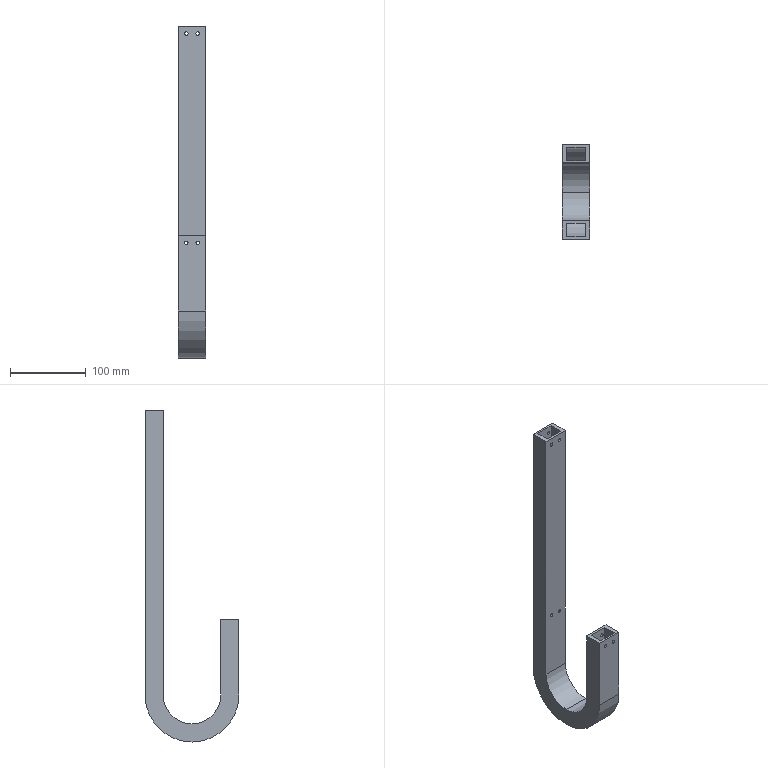Part | SolidWorks | features ICE 1, Sweep 1 | 1 solid | 46 faces | box 36 x 124 x 438 mm | volume 261522 mm3 | cylinder 32 | plane 14 | commonest cylinder face diameters 4.5 x24 76 x2 82 x2 118 x2 124 x2
STEP:
#1=CARTESIAN_POINT('',(7.5,91.,263.75));
#2=VERTEX_POINT('',#1);
#3=CARTESIAN_POINT('',(7.5,91.,268.25));
#4=VERTEX_POINT('',#3);
#5=CARTESIAN_POINT('',(7.5,91.,266.));
#6=DIRECTION('',(0.,1.,0.));
#7=DIRECTION('',(-1.,0.,0.));
#8=AXIS2_PLACEMENT_3D('',#5,#6,#7);
#9=CIRCLE('',#8,2.25);
#10=EDGE_CURVE('',#2,#4,#9,.T.);
#11=ORIENTED_EDGE('',*,*,#10,.T.);
#12=CARTESIAN_POINT('',(7.5,88.,268.25));
#13=VERTEX_POINT('',#12);
#14=CARTESIAN_POINT('',(7.5,112.,268.25));
#15=DIRECTION('',(0.,-1.,0.));
#16=VECTOR('',#15,1000.);
#17=LINE('',#14,#16);
#18=EDGE_CURVE('',#4,#13,#17,.T.);
#19=ORIENTED_EDGE('',*,*,#18,.T.);
#20=CARTESIAN_POINT('',(7.5,88.,263.75));
#21=VERTEX_POINT('',#20);
#22=CARTESIAN_POINT('',(7.5,88.,266.));
#23=DIRECTION('',(0.,1.,0.));
#24=DIRECTION('',(0.,0.,1.));
#25=AXIS2_PLACEMENT_3D('',#22,#23,#24);
#26=CIRCLE('',#25,2.25);
#27=EDGE_CURVE('',#21,#13,#26,.T.);
#28=ORIENTED_EDGE('',*,*,#27,.F.);
#29=CARTESIAN_POINT('',(7.5,112.,263.75));
#30=DIRECTION('',(0.,-1.,0.));
#31=VECTOR('',#30,1000.);
#32=LINE('',#29,#31);
#33=EDGE_CURVE('',#2,#21,#32,.T.);
#34=ORIENTED_EDGE('',*,*,#33,.F.);
#35=EDGE_LOOP('',(#11,#19,#28,#34));
#36=FACE_OUTER_BOUND('',#35,.T.);
#37=CARTESIAN_POINT('',(7.5,112.,266.));
#38=DIRECTION('',(0.,-1.,0.));
#39=DIRECTION('',(0.,0.,-1.));
#40=AXIS2_PLACEMENT_3D('',#37,#38,#39);
#41=CYLINDRICAL_SURFACE('',#40,2.25);
#42=ADVANCED_FACE('',(#36),#41,.F.);
#43=CARTESIAN_POINT('',(7.5,112.,268.25));
#44=VERTEX_POINT('',#43);
#45=CARTESIAN_POINT('',(7.5,112.,263.75));
#46=VERTEX_POINT('',#45);
#47=CARTESIAN_POINT('',(7.5,112.,266.));
#48=DIRECTION('',(0.,-1.,0.));
#49=DIRECTION('',(0.,0.,-1.));
#50=AXIS2_PLACEMENT_3D('',#47,#48,#49);
#51=CIRCLE('',#50,2.25);
#52=EDGE_CURVE('',#44,#46,#51,.T.);
#53=ORIENTED_EDGE('',*,*,#52,.F.);
#54=CARTESIAN_POINT('',(7.5,109.,268.25));
#55=VERTEX_POINT('',#54);
#56=CARTESIAN_POINT('',(7.5,112.,268.25));
#57=DIRECTION('',(0.,-1.,0.));
#58=VECTOR('',#57,1000.);
#59=LINE('',#56,#58);
#60=EDGE_CURVE('',#44,#55,#59,.T.);
#61=ORIENTED_EDGE('',*,*,#60,.T.);
#62=CARTESIAN_POINT('',(7.5,109.,263.75));
#63=VERTEX_POINT('',#62);
#64=CARTESIAN_POINT('',(7.5,109.,266.));
#65=DIRECTION('',(0.,-1.,0.));
#66=DIRECTION('',(0.,0.,-1.));
#67=AXIS2_PLACEMENT_3D('',#64,#65,#66);
#68=CIRCLE('',#67,2.25);
#69=EDGE_CURVE('',#55,#63,#68,.T.);
#70=ORIENTED_EDGE('',*,*,#69,.T.);
#71=CARTESIAN_POINT('',(7.5,112.,263.75));
#72=DIRECTION('',(0.,-1.,0.));
#73=VECTOR('',#72,1000.);
#74=LINE('',#71,#73);
#75=EDGE_CURVE('',#46,#63,#74,.T.);
#76=ORIENTED_EDGE('',*,*,#75,.F.);
#77=EDGE_LOOP('',(#53,#61,#70,#76));
#78=FACE_OUTER_BOUND('',#77,.T.);
#79=CARTESIAN_POINT('',(7.5,112.,266.));
#80=DIRECTION('',(0.,-1.,0.));
#81=DIRECTION('',(0.,0.,-1.));
#82=AXIS2_PLACEMENT_3D('',#79,#80,#81);
#83=CYLINDRICAL_SURFACE('',#82,2.25);
#84=ADVANCED_FACE('',(#78),#83,.F.);
#85=CARTESIAN_POINT('',(-7.5,91.,263.75));
#86=VERTEX_POINT('',#85);
#87=CARTESIAN_POINT('',(-7.5,91.,268.25));
#88=VERTEX_POINT('',#87);
#89=CARTESIAN_POINT('',(-7.5,91.,266.));
#90=DIRECTION('',(0.,1.,0.));
#91=DIRECTION('',(-1.,0.,0.));
#92=AXIS2_PLACEMENT_3D('',#89,#90,#91);
#93=CIRCLE('',#92,2.25);
#94=EDGE_CURVE('',#86,#88,#93,.T.);
#95=ORIENTED_EDGE('',*,*,#94,.T.);
#96=CARTESIAN_POINT('',(-7.5,88.,268.25));
#97=VERTEX_POINT('',#96);
#98=CARTESIAN_POINT('',(-7.5,112.,268.25));
#99=DIRECTION('',(0.,-1.,0.));
#100=VECTOR('',#99,1000.);
#101=LINE('',#98,#100);
#102=EDGE_CURVE('',#88,#97,#101,.T.);
#103=ORIENTED_EDGE('',*,*,#102,.T.);
#104=CARTESIAN_POINT('',(-7.5,88.,263.75));
#105=VERTEX_POINT('',#104);
#106=CARTESIAN_POINT('',(-7.5,88.,266.));
#107=DIRECTION('',(0.,1.,0.));
#108=DIRECTION('',(0.,0.,1.));
#109=AXIS2_PLACEMENT_3D('',#106,#107,#108);
#110=CIRCLE('',#109,2.25);
#111=EDGE_CURVE('',#105,#97,#110,.T.);
#112=ORIENTED_EDGE('',*,*,#111,.F.);
#113=CARTESIAN_POINT('',(-7.5,112.,263.75));
#114=DIRECTION('',(0.,-1.,0.));
#115=VECTOR('',#114,1000.);
#116=LINE('',#113,#115);
#117=EDGE_CURVE('',#86,#105,#116,.T.);
#118=ORIENTED_EDGE('',*,*,#117,.F.);
#119=EDGE_LOOP('',(#95,#103,#112,#118));
#120=FACE_OUTER_BOUND('',#119,.T.);
#121=CARTESIAN_POINT('',(-7.5,112.,266.));
#122=DIRECTION('',(0.,-1.,0.));
#123=DIRECTION('',(0.,0.,-1.));
#124=AXIS2_PLACEMENT_3D('',#121,#122,#123);
#125=CYLINDRICAL_SURFACE('',#124,2.25);
#126=ADVANCED_FACE('',(#120),#125,.F.);
#127=CARTESIAN_POINT('',(-7.5,112.,268.25));
#128=VERTEX_POINT('',#127);
#129=CARTESIAN_POINT('',(-7.5,112.,263.75));
#130=VERTEX_POINT('',#129);
#131=CARTESIAN_POINT('',(-7.5,112.,266.));
#132=DIRECTION('',(0.,-1.,0.));
#133=DIRECTION('',(0.,0.,-1.));
#134=AXIS2_PLACEMENT_3D('',#131,#132,#133);
#135=CIRCLE('',#134,2.25);
#136=EDGE_CURVE('',#128,#130,#135,.T.);
#137=ORIENTED_EDGE('',*,*,#136,.F.);
#138=CARTESIAN_POINT('',(-7.5,109.,268.25));
#139=VERTEX_POINT('',#138);
#140=CARTESIAN_POINT('',(-7.5,112.,268.25));
#141=DIRECTION('',(0.,-1.,0.));
#142=VECTOR('',#141,1000.);
#143=LINE('',#140,#142);
#144=EDGE_CURVE('',#128,#139,#143,.T.);
#145=ORIENTED_EDGE('',*,*,#144,.T.);
#146=CARTESIAN_POINT('',(-7.5,109.,263.75));
#147=VERTEX_POINT('',#146);
#148=CARTESIAN_POINT('',(-7.5,109.,266.));
#149=DIRECTION('',(0.,-1.,0.));
#150=DIRECTION('',(0.,0.,-1.));
#151=AXIS2_PLACEMENT_3D('',#148,#149,#150);
#152=CIRCLE('',#151,2.25);
#153=EDGE_CURVE('',#139,#147,#152,.T.);
#154=ORIENTED_EDGE('',*,*,#153,.T.);
#155=CARTESIAN_POINT('',(-7.5,112.,263.75));
#156=DIRECTION('',(0.,-1.,0.));
#157=VECTOR('',#156,1000.);
#158=LINE('',#155,#157);
#159=EDGE_CURVE('',#130,#147,#158,.T.);
#160=ORIENTED_EDGE('',*,*,#159,.F.);
#161=EDGE_LOOP('',(#137,#145,#154,#160));
#162=FACE_OUTER_BOUND('',#161,.T.);
#163=CARTESIAN_POINT('',(-7.5,112.,266.));
#164=DIRECTION('',(0.,-1.,0.));
#165=DIRECTION('',(0.,0.,-1.));
#166=AXIS2_PLACEMENT_3D('',#163,#164,#165);
#167=CYLINDRICAL_SURFACE('',#166,2.25);
#168=ADVANCED_FACE('',(#162),#167,.F.);
#169=CARTESIAN_POINT('',(7.5,91.,-12.25));
#170=VERTEX_POINT('',#169);
#171=CARTESIAN_POINT('',(7.5,91.,-7.75));
#172=VERTEX_POINT('',#171);
#173=CARTESIAN_POINT('',(7.5,91.,-10.));
#174=DIRECTION('',(0.,1.,0.));
#175=DIRECTION('',(-1.,0.,0.));
#176=AXIS2_PLACEMENT_3D('',#173,#174,#175);
#177=CIRCLE('',#176,2.25);
#178=EDGE_CURVE('',#170,#172,#177,.T.);
#179=ORIENTED_EDGE('',*,*,#178,.T.);
#180=CARTESIAN_POINT('',(7.5,88.,-7.75));
#181=VERTEX_POINT('',#180);
#182=CARTESIAN_POINT('',(7.5,112.,-7.75));
#183=DIRECTION('',(0.,-1.,0.));
#184=VECTOR('',#183,1000.);
#185=LINE('',#182,#184);
#186=EDGE_CURVE('',#172,#181,#185,.T.);
#187=ORIENTED_EDGE('',*,*,#186,.T.);
#188=CARTESIAN_POINT('',(7.5,88.,-12.25));
#189=VERTEX_POINT('',#188);
#190=CARTESIAN_POINT('',(7.5,88.,-10.));
#191=DIRECTION('',(0.,1.,0.));
#192=DIRECTION('',(0.,0.,1.));
#193=AXIS2_PLACEMENT_3D('',#190,#191,#192);
#194=CIRCLE('',#193,2.25);
#195=EDGE_CURVE('',#189,#181,#194,.T.);
#196=ORIENTED_EDGE('',*,*,#195,.F.);
#197=CARTESIAN_POINT('',(7.5,112.,-12.25));
#198=DIRECTION('',(0.,-1.,0.));
#199=VECTOR('',#198,1000.);
#200=LINE('',#197,#199);
#201=EDGE_CURVE('',#170,#189,#200,.T.);
#202=ORIENTED_EDGE('',*,*,#201,.F.);
#203=EDGE_LOOP('',(#179,#187,#196,#202));
#204=FACE_OUTER_BOUND('',#203,.T.);
#205=CARTESIAN_POINT('',(7.5,112.,-10.));
#206=DIRECTION('',(0.,-1.,0.));
#207=DIRECTION('',(0.,0.,-1.));
#208=AXIS2_PLACEMENT_3D('',#205,#206,#207);
#209=CYLINDRICAL_SURFACE('',#208,2.25);
#210=ADVANCED_FACE('',(#204),#209,.F.);
#211=CARTESIAN_POINT('',(7.5,112.,-7.75));
#212=VERTEX_POINT('',#211);
#213=CARTESIAN_POINT('',(7.5,112.,-12.25));
#214=VERTEX_POINT('',#213);
#215=CARTESIAN_POINT('',(7.5,112.,-10.));
#216=DIRECTION('',(0.,-1.,0.));
#217=DIRECTION('',(0.,0.,-1.));
#218=AXIS2_PLACEMENT_3D('',#215,#216,#217);
#219=CIRCLE('',#218,2.25);
#220=EDGE_CURVE('',#212,#214,#219,.T.);
#221=ORIENTED_EDGE('',*,*,#220,.F.);
#222=CARTESIAN_POINT('',(7.5,109.,-7.75));
#223=VERTEX_POINT('',#222);
#224=CARTESIAN_POINT('',(7.5,112.,-7.75));
#225=DIRECTION('',(0.,-1.,0.));
#226=VECTOR('',#225,1000.);
#227=LINE('',#224,#226);
#228=EDGE_CURVE('',#212,#223,#227,.T.);
#229=ORIENTED_EDGE('',*,*,#228,.T.);
#230=CARTESIAN_POINT('',(7.5,109.,-12.25));
#231=VERTEX_POINT('',#230);
#232=CARTESIAN_POINT('',(7.5,109.,-10.));
#233=DIRECTION('',(0.,-1.,0.));
#234=DIRECTION('',(0.,0.,-1.));
#235=AXIS2_PLACEMENT_3D('',#232,#233,#234);
#236=CIRCLE('',#235,2.25);
#237=EDGE_CURVE('',#223,#231,#236,.T.);
#238=ORIENTED_EDGE('',*,*,#237,.T.);
#239=CARTESIAN_POINT('',(7.5,112.,-12.25));
#240=DIRECTION('',(0.,-1.,0.));
#241=VECTOR('',#240,1000.);
#242=LINE('',#239,#241);
#243=EDGE_CURVE('',#214,#231,#242,.T.);
#244=ORIENTED_EDGE('',*,*,#243,.F.);
#245=EDGE_LOOP('',(#221,#229,#238,#244));
#246=FACE_OUTER_BOUND('',#245,.T.);
#247=CARTESIAN_POINT('',(7.5,112.,-10.));
#248=DIRECTION('',(0.,-1.,0.));
#249=DIRECTION('',(0.,0.,-1.));
#250=AXIS2_PLACEMENT_3D('',#247,#248,#249);
#251=CYLINDRICAL_SURFACE('',#250,2.25);
#252=ADVANCED_FACE('',(#246),#251,.F.);
#253=CARTESIAN_POINT('',(7.5,-9.,-7.75));
#254=VERTEX_POINT('',#253);
#255=CARTESIAN_POINT('',(7.5,-9.,-12.25));
#256=VERTEX_POINT('',#255);
#257=CARTESIAN_POINT('',(7.5,-9.,-10.));
#258=DIRECTION('',(0.,-1.,0.));
#259=DIRECTION('',(0.,0.,-1.));
#260=AXIS2_PLACEMENT_3D('',#257,#258,#259);
#261=CIRCLE('',#260,2.25);
#262=EDGE_CURVE('',#254,#256,#261,.T.);
#263=ORIENTED_EDGE('',*,*,#262,.F.);
#264=CARTESIAN_POINT('',(7.5,-12.,-7.75));
#265=VERTEX_POINT('',#264);
#266=CARTESIAN_POINT('',(7.5,112.,-7.75));
#267=DIRECTION('',(0.,-1.,0.));
#268=VECTOR('',#267,1000.);
#269=LINE('',#266,#268);
#270=EDGE_CURVE('',#254,#265,#269,.T.);
#271=ORIENTED_EDGE('',*,*,#270,.T.);
#272=CARTESIAN_POINT('',(7.5,-12.,-12.25));
#273=VERTEX_POINT('',#272);
#274=CARTESIAN_POINT('',(7.5,-12.,-10.));
#275=DIRECTION('',(0.,-1.,0.));
#276=DIRECTION('',(0.,0.,-1.));
#277=AXIS2_PLACEMENT_3D('',#274,#275,#276);
#278=CIRCLE('',#277,2.25);
#279=EDGE_CURVE('',#265,#273,#278,.T.);
#280=ORIENTED_EDGE('',*,*,#279,.T.);
#281=CARTESIAN_POINT('',(7.5,112.,-12.25));
#282=DIRECTION('',(0.,-1.,0.));
#283=VECTOR('',#282,1000.);
#284=LINE('',#281,#283);
#285=EDGE_CURVE('',#256,#273,#284,.T.);
#286=ORIENTED_EDGE('',*,*,#285,.F.);
#287=EDGE_LOOP('',(#263,#271,#280,#286));
#288=FACE_OUTER_BOUND('',#287,.T.);
#289=CARTESIAN_POINT('',(7.5,112.,-10.));
#290=DIRECTION('',(0.,-1.,0.));
#291=DIRECTION('',(0.,0.,-1.));
#292=AXIS2_PLACEMENT_3D('',#289,#290,#291);
#293=CYLINDRICAL_SURFACE('',#292,2.25);
#294=ADVANCED_FACE('',(#288),#293,.F.);
#295=CARTESIAN_POINT('',(7.5,12.,-12.25));
#296=VERTEX_POINT('',#295);
#297=CARTESIAN_POINT('',(7.5,12.,-7.75));
#298=VERTEX_POINT('',#297);
#299=CARTESIAN_POINT('',(7.5,12.,-10.));
#300=DIRECTION('',(0.,1.,0.));
#301=DIRECTION('',(0.,0.,1.));
#302=AXIS2_PLACEMENT_3D('',#299,#300,#301);
#303=CIRCLE('',#302,2.25);
#304=EDGE_CURVE('',#296,#298,#303,.T.);
#305=ORIENTED_EDGE('',*,*,#304,.T.);
#306=CARTESIAN_POINT('',(7.5,9.,-7.75));
#307=VERTEX_POINT('',#306);
#308=CARTESIAN_POINT('',(7.5,112.,-7.75));
#309=DIRECTION('',(0.,-1.,0.));
#310=VECTOR('',#309,1000.);
#311=LINE('',#308,#310);
#312=EDGE_CURVE('',#298,#307,#311,.T.);
#313=ORIENTED_EDGE('',*,*,#312,.T.);
#314=CARTESIAN_POINT('',(7.5,9.,-12.25));
#315=VERTEX_POINT('',#314);
#316=CARTESIAN_POINT('',(7.5,9.,-10.));
#317=DIRECTION('',(0.,1.,0.));
#318=DIRECTION('',(-1.,0.,0.));
#319=AXIS2_PLACEMENT_3D('',#316,#317,#318);
#320=CIRCLE('',#319,2.25);
#321=EDGE_CURVE('',#315,#307,#320,.T.);
#322=ORIENTED_EDGE('',*,*,#321,.F.);
#323=CARTESIAN_POINT('',(7.5,112.,-12.25));
#324=DIRECTION('',(0.,-1.,0.));
#325=VECTOR('',#324,1000.);
#326=LINE('',#323,#325);
#327=EDGE_CURVE('',#296,#315,#326,.T.);
#328=ORIENTED_EDGE('',*,*,#327,.F.);
#329=EDGE_LOOP('',(#305,#313,#322,#328));
#330=FACE_OUTER_BOUND('',#329,.T.);
#331=CARTESIAN_POINT('',(7.5,112.,-10.));
#332=DIRECTION('',(0.,-1.,0.));
#333=DIRECTION('',(0.,0.,-1.));
#334=AXIS2_PLACEMENT_3D('',#331,#332,#333);
#335=CYLINDRICAL_SURFACE('',#334,2.25);
#336=ADVANCED_FACE('',(#330),#335,.F.);
#337=CARTESIAN_POINT('',(-7.5,91.,-12.25));
#338=VERTEX_POINT('',#337);
#339=CARTESIAN_POINT('',(-7.5,91.,-7.75));
#340=VERTEX_POINT('',#339);
#341=CARTESIAN_POINT('',(-7.5,91.,-10.));
#342=DIRECTION('',(0.,1.,0.));
#343=DIRECTION('',(-1.,0.,0.));
#344=AXIS2_PLACEMENT_3D('',#341,#342,#343);
#345=CIRCLE('',#344,2.25);
#346=EDGE_CURVE('',#338,#340,#345,.T.);
#347=ORIENTED_EDGE('',*,*,#346,.T.);
#348=CARTESIAN_POINT('',(-7.5,88.,-7.75));
#349=VERTEX_POINT('',#348);
#350=CARTESIAN_POINT('',(-7.5,112.,-7.75));
#351=DIRECTION('',(0.,-1.,0.));
#352=VECTOR('',#351,1000.);
#353=LINE('',#350,#352);
#354=EDGE_CURVE('',#340,#349,#353,.T.);
#355=ORIENTED_EDGE('',*,*,#354,.T.);
#356=CARTESIAN_POINT('',(-7.5,88.,-12.25));
#357=VERTEX_POINT('',#356);
#358=CARTESIAN_POINT('',(-7.5,88.,-10.));
#359=DIRECTION('',(0.,1.,0.));
#360=DIRECTION('',(0.,0.,1.));
#361=AXIS2_PLACEMENT_3D('',#358,#359,#360);
#362=CIRCLE('',#361,2.25);
#363=EDGE_CURVE('',#357,#349,#362,.T.);
#364=ORIENTED_EDGE('',*,*,#363,.F.);
#365=CARTESIAN_POINT('',(-7.5,112.,-12.25));
#366=DIRECTION('',(0.,-1.,0.));
#367=VECTOR('',#366,1000.);
#368=LINE('',#365,#367);
#369=EDGE_CURVE('',#338,#357,#368,.T.);
#370=ORIENTED_EDGE('',*,*,#369,.F.);
#371=EDGE_LOOP('',(#347,#355,#364,#370));
#372=FACE_OUTER_BOUND('',#371,.T.);
#373=CARTESIAN_POINT('',(-7.5,112.,-10.));
#374=DIRECTION('',(0.,-1.,0.));
#375=DIRECTION('',(0.,0.,-1.));
#376=AXIS2_PLACEMENT_3D('',#373,#374,#375);
#377=CYLINDRICAL_SURFACE('',#376,2.25);
#378=ADVANCED_FACE('',(#372),#377,.F.);
#379=CARTESIAN_POINT('',(-7.5,112.,-7.75));
#380=VERTEX_POINT('',#379);
#381=CARTESIAN_POINT('',(-7.5,112.,-12.25));
#382=VERTEX_POINT('',#381);
#383=CARTESIAN_POINT('',(-7.5,112.,-10.));
#384=DIRECTION('',(0.,-1.,0.));
#385=DIRECTION('',(0.,0.,-1.));
#386=AXIS2_PLACEMENT_3D('',#383,#384,#385);
#387=CIRCLE('',#386,2.25);
#388=EDGE_CURVE('',#380,#382,#387,.T.);
#389=ORIENTED_EDGE('',*,*,#388,.F.);
#390=CARTESIAN_POINT('',(-7.5,109.,-7.75));
#391=VERTEX_POINT('',#390);
#392=CARTESIAN_POINT('',(-7.5,112.,-7.75));
#393=DIRECTION('',(0.,-1.,0.));
#394=VECTOR('',#393,1000.);
#395=LINE('',#392,#394);
#396=EDGE_CURVE('',#380,#391,#395,.T.);
#397=ORIENTED_EDGE('',*,*,#396,.T.);
#398=CARTESIAN_POINT('',(-7.5,109.,-12.25));
#399=VERTEX_POINT('',#398);
#400=CARTESIAN_POINT('',(-7.5,109.,-10.));
#401=DIRECTION('',(0.,-1.,0.));
#402=DIRECTION('',(0.,0.,-1.));
#403=AXIS2_PLACEMENT_3D('',#400,#401,#402);
#404=CIRCLE('',#403,2.25);
#405=EDGE_CURVE('',#391,#399,#404,.T.);
#406=ORIENTED_EDGE('',*,*,#405,.T.);
#407=CARTESIAN_POINT('',(-7.5,112.,-12.25));
#408=DIRECTION('',(0.,-1.,0.));
#409=VECTOR('',#408,1000.);
#410=LINE('',#407,#409);
#411=EDGE_CURVE('',#382,#399,#410,.T.);
#412=ORIENTED_EDGE('',*,*,#411,.F.);
#413=EDGE_LOOP('',(#389,#397,#406,#412));
#414=FACE_OUTER_BOUND('',#413,.T.);
#415=CARTESIAN_POINT('',(-7.5,112.,-10.));
#416=DIRECTION('',(0.,-1.,0.));
#417=DIRECTION('',(0.,0.,-1.));
#418=AXIS2_PLACEMENT_3D('',#415,#416,#417);
#419=CYLINDRICAL_SURFACE('',#418,2.25);
#420=ADVANCED_FACE('',(#414),#419,.F.);
#421=CARTESIAN_POINT('',(-7.5,-9.,-7.75));
#422=VERTEX_POINT('',#421);
#423=CARTESIAN_POINT('',(-7.5,-9.,-12.25));
#424=VERTEX_POINT('',#423);
#425=CARTESIAN_POINT('',(-7.5,-9.,-10.));
#426=DIRECTION('',(0.,-1.,0.));
#427=DIRECTION('',(0.,0.,-1.));
#428=AXIS2_PLACEMENT_3D('',#425,#426,#427);
#429=CIRCLE('',#428,2.25);
#430=EDGE_CURVE('',#422,#424,#429,.T.);
#431=ORIENTED_EDGE('',*,*,#430,.F.);
#432=CARTESIAN_POINT('',(-7.5,-12.,-7.75));
#433=VERTEX_POINT('',#432);
#434=CARTESIAN_POINT('',(-7.5,112.,-7.75));
#435=DIRECTION('',(0.,-1.,0.));
#436=VECTOR('',#435,1000.);
#437=LINE('',#434,#436);
#438=EDGE_CURVE('',#422,#433,#437,.T.);
#439=ORIENTED_EDGE('',*,*,#438,.T.);
#440=CARTESIAN_POINT('',(-7.5,-12.,-12.25));
#441=VERTEX_POINT('',#440);
#442=CARTESIAN_POINT('',(-7.5,-12.,-10.));
#443=DIRECTION('',(0.,-1.,0.));
#444=DIRECTION('',(0.,0.,-1.));
#445=AXIS2_PLACEMENT_3D('',#442,#443,#444);
#446=CIRCLE('',#445,2.25);
#447=EDGE_CURVE('',#433,#441,#446,.T.);
#448=ORIENTED_EDGE('',*,*,#447,.T.);
#449=CARTESIAN_POINT('',(-7.5,112.,-12.25));
#450=DIRECTION('',(0.,-1.,0.));
#451=VECTOR('',#450,1000.);
#452=LINE('',#449,#451);
#453=EDGE_CURVE('',#424,#441,#452,.T.);
#454=ORIENTED_EDGE('',*,*,#453,.F.);
#455=EDGE_LOOP('',(#431,#439,#448,#454));
#456=FACE_OUTER_BOUND('',#455,.T.);
#457=CARTESIAN_POINT('',(-7.5,112.,-10.));
#458=DIRECTION('',(0.,-1.,0.));
#459=DIRECTION('',(0.,0.,-1.));
#460=AXIS2_PLACEMENT_3D('',#457,#458,#459);
#461=CYLINDRICAL_SURFACE('',#460,2.25);
#462=ADVANCED_FACE('',(#456),#461,.F.);
#463=CARTESIAN_POINT('',(-7.5,12.,-12.25));
#464=VERTEX_POINT('',#463);
#465=CARTESIAN_POINT('',(-7.5,12.,-7.75));
#466=VERTEX_POINT('',#465);
#467=CARTESIAN_POINT('',(-7.5,12.,-10.));
#468=DIRECTION('',(0.,1.,0.));
#469=DIRECTION('',(0.,0.,1.));
#470=AXIS2_PLACEMENT_3D('',#467,#468,#469);
#471=CIRCLE('',#470,2.25);
#472=EDGE_CURVE('',#464,#466,#471,.T.);
#473=ORIENTED_EDGE('',*,*,#472,.T.);
#474=CARTESIAN_POINT('',(-7.5,9.,-7.75));
#475=VERTEX_POINT('',#474);
#476=CARTESIAN_POINT('',(-7.5,112.,-7.75));
#477=DIRECTION('',(0.,-1.,0.));
#478=VECTOR('',#477,1000.);
#479=LINE('',#476,#478);
#480=EDGE_CURVE('',#466,#475,#479,.T.);
#481=ORIENTED_EDGE('',*,*,#480,.T.);
#482=CARTESIAN_POINT('',(-7.5,9.,-12.25));
#483=VERTEX_POINT('',#482);
#484=CARTESIAN_POINT('',(-7.5,9.,-10.));
#485=DIRECTION('',(0.,1.,0.));
#486=DIRECTION('',(-1.,0.,0.));
#487=AXIS2_PLACEMENT_3D('',#484,#485,#486);
#488=CIRCLE('',#487,2.25);
#489=EDGE_CURVE('',#483,#475,#488,.T.);
#490=ORIENTED_EDGE('',*,*,#489,.F.);
#491=CARTESIAN_POINT('',(-7.5,112.,-12.25));
#492=DIRECTION('',(0.,-1.,0.));
#493=VECTOR('',#492,1000.);
#494=LINE('',#491,#493);
#495=EDGE_CURVE('',#464,#483,#494,.T.);
#496=ORIENTED_EDGE('',*,*,#495,.F.);
#497=EDGE_LOOP('',(#473,#481,#490,#496));
#498=FACE_OUTER_BOUND('',#497,.T.);
#499=CARTESIAN_POINT('',(-7.5,112.,-10.));
#500=DIRECTION('',(0.,-1.,0.));
#501=DIRECTION('',(0.,0.,-1.));
#502=AXIS2_PLACEMENT_3D('',#499,#500,#501);
#503=CYLINDRICAL_SURFACE('',#502,2.25);
#504=ADVANCED_FACE('',(#498),#503,.F.);
#505=CARTESIAN_POINT('',(-12.5,50.,-159.));
#506=VERTEX_POINT('',#505);
#507=CARTESIAN_POINT('',(-12.5,109.,-100.));
#508=VERTEX_POINT('',#507);
#509=CARTESIAN_POINT('',(-12.5,50.,-100.));
#510=DIRECTION('',(1.,0.,0.));
#511=DIRECTION('',(0.,0.,-1.));
#512=AXIS2_PLACEMENT_3D('',#509,#510,#511);
#513=CIRCLE('',#512,59.);
#514=EDGE_CURVE('',#506,#508,#513,.T.);
#515=ORIENTED_EDGE('',*,*,#514,.F.);
#516=CARTESIAN_POINT('',(12.5,50.,-159.));
#517=VERTEX_POINT('',#516);
#518=CARTESIAN_POINT('',(0.,50.,-159.));
#519=DIRECTION('',(1.,0.,0.));
#520=VECTOR('',#519,1000.);
#521=LINE('',#518,#520);
#522=EDGE_CURVE('',#506,#517,#521,.T.);
#523=ORIENTED_EDGE('',*,*,#522,.T.);
#524=CARTESIAN_POINT('',(12.5,109.,-100.));
#525=VERTEX_POINT('',#524);
#526=CARTESIAN_POINT('',(12.5,50.,-100.));
#527=DIRECTION('',(1.,0.,0.));
#528=DIRECTION('',(0.,0.,-1.));
#529=AXIS2_PLACEMENT_3D('',#526,#527,#528);
#530=CIRCLE('',#529,59.);
#531=EDGE_CURVE('',#517,#525,#530,.T.);
#532=ORIENTED_EDGE('',*,*,#531,.T.);
#533=CARTESIAN_POINT('',(-12.5,109.,-100.));
#534=DIRECTION('',(1.,0.,0.));
#535=VECTOR('',#534,1000.);
#536=LINE('',#533,#535);
#537=EDGE_CURVE('',#508,#525,#536,.T.);
#538=ORIENTED_EDGE('',*,*,#537,.F.);
#539=EDGE_LOOP('',(#515,#523,#532,#538));
#540=FACE_OUTER_BOUND('',#539,.T.);
#541=CARTESIAN_POINT('',(0.,50.,-100.));
#542=DIRECTION('',(1.,0.,0.));
#543=DIRECTION('',(0.,0.,-1.));
#544=AXIS2_PLACEMENT_3D('',#541,#542,#543);
#545=CYLINDRICAL_SURFACE('',#544,59.);
#546=ADVANCED_FACE('',(#540),#545,.F.);
#547=CARTESIAN_POINT('',(-12.5,9.,-100.));
#548=VERTEX_POINT('',#547);
#549=CARTESIAN_POINT('',(-12.5,50.,-141.));
#550=VERTEX_POINT('',#549);
#551=CARTESIAN_POINT('',(-12.5,50.,-100.));
#552=DIRECTION('',(1.,0.,0.));
#553=DIRECTION('',(0.,0.,-1.));
#554=AXIS2_PLACEMENT_3D('',#551,#552,#553);
#555=CIRCLE('',#554,41.);
#556=EDGE_CURVE('',#548,#550,#555,.T.);
#557=ORIENTED_EDGE('',*,*,#556,.T.);
#558=CARTESIAN_POINT('',(12.5,50.,-141.));
#559=VERTEX_POINT('',#558);
#560=CARTESIAN_POINT('',(0.,50.,-141.));
#561=DIRECTION('',(1.,0.,0.));
#562=VECTOR('',#561,1000.);
#563=LINE('',#560,#562);
#564=EDGE_CURVE('',#550,#559,#563,.T.);
#565=ORIENTED_EDGE('',*,*,#564,.T.);
#566=CARTESIAN_POINT('',(12.5,9.,-100.));
#567=VERTEX_POINT('',#566);
#568=CARTESIAN_POINT('',(12.5,50.,-100.));
#569=DIRECTION('',(1.,0.,0.));
#570=DIRECTION('',(0.,0.,-1.));
#571=AXIS2_PLACEMENT_3D('',#568,#569,#570);
#572=CIRCLE('',#571,41.);
#573=EDGE_CURVE('',#567,#559,#572,.T.);
#574=ORIENTED_EDGE('',*,*,#573,.F.);
#575=CARTESIAN_POINT('',(-12.5,9.,-100.));
#576=DIRECTION('',(-1.,0.,0.));
#577=VECTOR('',#576,1000.);
#578=LINE('',#575,#577);
#579=EDGE_CURVE('',#567,#548,#578,.T.);
#580=ORIENTED_EDGE('',*,*,#579,.T.);
#581=EDGE_LOOP('',(#557,#565,#574,#580));
#582=FACE_OUTER_BOUND('',#581,.T.);
#583=CARTESIAN_POINT('',(0.,50.,-100.));
#584=DIRECTION('',(1.,0.,0.));
#585=DIRECTION('',(0.,0.,-1.));
#586=AXIS2_PLACEMENT_3D('',#583,#584,#585);
#587=CYLINDRICAL_SURFACE('',#586,41.);
#588=ADVANCED_FACE('',(#582),#587,.T.);
#589=CARTESIAN_POINT('',(-18.,50.,-138.));
#590=VERTEX_POINT('',#589);
#591=CARTESIAN_POINT('',(-18.,88.,-100.));
#592=VERTEX_POINT('',#591);
#593=CARTESIAN_POINT('',(-18.,50.,-100.));
#594=DIRECTION('',(1.,0.,0.));
#595=DIRECTION('',(0.,0.,-1.));
#596=AXIS2_PLACEMENT_3D('',#593,#594,#595);
#597=CIRCLE('',#596,38.);
#598=EDGE_CURVE('',#590,#592,#597,.T.);
#599=ORIENTED_EDGE('',*,*,#598,.F.);
#600=CARTESIAN_POINT('',(18.,50.,-138.));
#601=VERTEX_POINT('',#600);
#602=CARTESIAN_POINT('',(0.,50.,-138.));
#603=DIRECTION('',(1.,0.,0.));
#604=VECTOR('',#603,1000.);
#605=LINE('',#602,#604);
#606=EDGE_CURVE('',#590,#601,#605,.T.);
#607=ORIENTED_EDGE('',*,*,#606,.T.);
#608=CARTESIAN_POINT('',(18.,88.,-100.));
#609=VERTEX_POINT('',#608);
#610=CARTESIAN_POINT('',(18.,50.,-100.));
#611=DIRECTION('',(1.,0.,0.));
#612=DIRECTION('',(0.,0.,-1.));
#613=AXIS2_PLACEMENT_3D('',#610,#611,#612);
#614=CIRCLE('',#613,38.);
#615=EDGE_CURVE('',#601,#609,#614,.T.);
#616=ORIENTED_EDGE('',*,*,#615,.T.);
#617=CARTESIAN_POINT('',(-18.,88.,-100.));
#618=DIRECTION('',(-1.,0.,0.));
#619=VECTOR('',#618,1000.);
#620=LINE('',#617,#619);
#621=EDGE_CURVE('',#609,#592,#620,.T.);
#622=ORIENTED_EDGE('',*,*,#621,.T.);
#623=EDGE_LOOP('',(#599,#607,#616,#622));
#624=FACE_OUTER_BOUND('',#623,.T.);
#625=CARTESIAN_POINT('',(0.,50.,-100.));
#626=DIRECTION('',(1.,0.,0.));
#627=DIRECTION('',(0.,0.,-1.));
#628=AXIS2_PLACEMENT_3D('',#625,#626,#627);
#629=CYLINDRICAL_SURFACE('',#628,38.);
#630=ADVANCED_FACE('',(#624),#629,.F.);
#631=CARTESIAN_POINT('',(-18.,-12.,-100.));
#632=VERTEX_POINT('',#631);
#633=CARTESIAN_POINT('',(-18.,50.,-162.));
#634=VERTEX_POINT('',#633);
#635=CARTESIAN_POINT('',(-18.,50.,-100.));
#636=DIRECTION('',(1.,0.,0.));
#637=DIRECTION('',(0.,0.,-1.));
#638=AXIS2_PLACEMENT_3D('',#635,#636,#637);
#639=CIRCLE('',#638,62.);
#640=EDGE_CURVE('',#632,#634,#639,.T.);
#641=ORIENTED_EDGE('',*,*,#640,.T.);
#642=CARTESIAN_POINT('',(18.,50.,-162.));
#643=VERTEX_POINT('',#642);
#644=CARTESIAN_POINT('',(0.,50.,-162.));
#645=DIRECTION('',(1.,0.,0.));
#646=VECTOR('',#645,1000.);
#647=LINE('',#644,#646);
#648=EDGE_CURVE('',#634,#643,#647,.T.);
#649=ORIENTED_EDGE('',*,*,#648,.T.);
#650=CARTESIAN_POINT('',(18.,-12.,-100.));
#651=VERTEX_POINT('',#650);
#652=CARTESIAN_POINT('',(18.,50.,-100.));
#653=DIRECTION('',(1.,0.,0.));
#654=DIRECTION('',(0.,0.,-1.));
#655=AXIS2_PLACEMENT_3D('',#652,#653,#654);
#656=CIRCLE('',#655,62.);
#657=EDGE_CURVE('',#651,#643,#656,.T.);
#658=ORIENTED_EDGE('',*,*,#657,.F.);
#659=CARTESIAN_POINT('',(-18.,-12.,-100.));
#660=DIRECTION('',(1.,0.,0.));
#661=VECTOR('',#660,1000.);
#662=LINE('',#659,#661);
#663=EDGE_CURVE('',#632,#651,#662,.T.);
#664=ORIENTED_EDGE('',*,*,#663,.F.);
#665=EDGE_LOOP('',(#641,#649,#658,#664));
#666=FACE_OUTER_BOUND('',#665,.T.);
#667=CARTESIAN_POINT('',(0.,50.,-100.));
#668=DIRECTION('',(1.,0.,0.));
#669=DIRECTION('',(0.,0.,-1.));
#670=AXIS2_PLACEMENT_3D('',#667,#668,#669);
#671=CYLINDRICAL_SURFACE('',#670,62.);
#672=ADVANCED_FACE('',(#666),#671,.T.);
#673=CARTESIAN_POINT('',(7.5,112.,266.));
#674=DIRECTION('',(0.,-1.,0.));
#675=DIRECTION('',(0.,0.,-1.));
#676=AXIS2_PLACEMENT_3D('',#673,#674,#675);
#677=CIRCLE('',#676,2.25);
#678=EDGE_CURVE('',#46,#44,#677,.T.);
#679=ORIENTED_EDGE('',*,*,#678,.T.);
#680=ORIENTED_EDGE('',*,*,#52,.T.);
#681=EDGE_LOOP('',(#679,#680));
#682=FACE_BOUND('',#681,.T.);
#683=CARTESIAN_POINT('',(-7.5,112.,266.));
#684=DIRECTION('',(0.,-1.,0.));
#685=DIRECTION('',(0.,0.,-1.));
#686=AXIS2_PLACEMENT_3D('',#683,#684,#685);
#687=CIRCLE('',#686,2.25);
#688=EDGE_CURVE('',#130,#128,#687,.T.);
#689=ORIENTED_EDGE('',*,*,#688,.T.);
#690=ORIENTED_EDGE('',*,*,#136,.T.);
#691=EDGE_LOOP('',(#689,#690));
#692=FACE_BOUND('',#691,.T.);
#693=CARTESIAN_POINT('',(7.5,112.,-10.));
#694=DIRECTION('',(0.,-1.,0.));
#695=DIRECTION('',(0.,0.,-1.));
#696=AXIS2_PLACEMENT_3D('',#693,#694,#695);
#697=CIRCLE('',#696,2.25);
#698=EDGE_CURVE('',#214,#212,#697,.T.);
#699=ORIENTED_EDGE('',*,*,#698,.T.);
#700=ORIENTED_EDGE('',*,*,#220,.T.);
#701=EDGE_LOOP('',(#699,#700));
#702=FACE_BOUND('',#701,.T.);
#703=CARTESIAN_POINT('',(-7.5,112.,-10.));
#704=DIRECTION('',(0.,-1.,0.));
#705=DIRECTION('',(0.,0.,-1.));
#706=AXIS2_PLACEMENT_3D('',#703,#704,#705);
#707=CIRCLE('',#706,2.25);
#708=EDGE_CURVE('',#382,#380,#707,.T.);
#709=ORIENTED_EDGE('',*,*,#708,.T.);
#710=ORIENTED_EDGE('',*,*,#388,.T.);
#711=EDGE_LOOP('',(#709,#710));
#712=FACE_BOUND('',#711,.T.);
#713=CARTESIAN_POINT('',(-18.,112.,-100.));
#714=VERTEX_POINT('',#713);
#715=CARTESIAN_POINT('',(18.,112.,-100.));
#716=VERTEX_POINT('',#715);
#717=CARTESIAN_POINT('',(-18.,112.,-100.));
#718=DIRECTION('',(1.,0.,0.));
#719=VECTOR('',#718,1000.);
#720=LINE('',#717,#719);
#721=EDGE_CURVE('',#714,#716,#720,.T.);
#722=ORIENTED_EDGE('',*,*,#721,.F.);
#723=CARTESIAN_POINT('',(-18.,112.,276.));
#724=VERTEX_POINT('',#723);
#725=CARTESIAN_POINT('',(-18.,112.,-100.));
#726=DIRECTION('',(0.,0.,1.));
#727=VECTOR('',#726,1000.);
#728=LINE('',#725,#727);
#729=EDGE_CURVE('',#714,#724,#728,.T.);
#730=ORIENTED_EDGE('',*,*,#729,.T.);
#731=CARTESIAN_POINT('',(18.,112.,276.));
#732=VERTEX_POINT('',#731);
#733=CARTESIAN_POINT('',(-18.,112.,276.));
#734=DIRECTION('',(1.,0.,0.));
#735=VECTOR('',#734,1000.);
#736=LINE('',#733,#735);
#737=EDGE_CURVE('',#724,#732,#736,.T.);
#738=ORIENTED_EDGE('',*,*,#737,.T.);
#739=CARTESIAN_POINT('',(18.,112.,-100.));
#740=DIRECTION('',(0.,0.,1.));
#741=VECTOR('',#740,1000.);
#742=LINE('',#739,#741);
#743=EDGE_CURVE('',#716,#732,#742,.T.);
#744=ORIENTED_EDGE('',*,*,#743,.F.);
#745=EDGE_LOOP('',(#722,#730,#738,#744));
#746=FACE_OUTER_BOUND('',#745,.T.);
#747=CARTESIAN_POINT('',(-18.,112.,-100.));
#748=DIRECTION('',(0.,-1.,0.));
#749=DIRECTION('',(0.,0.,-1.));
#750=AXIS2_PLACEMENT_3D('',#747,#748,#749);
#751=PLANE('',#750);
#752=ADVANCED_FACE('',(#682,#692,#702,#712,#746),#751,.F.);
#753=ORIENTED_EDGE('',*,*,#27,.T.);
#754=CARTESIAN_POINT('',(7.5,88.,266.));
#755=DIRECTION('',(0.,1.,0.));
#756=DIRECTION('',(0.,0.,1.));
#757=AXIS2_PLACEMENT_3D('',#754,#755,#756);
#758=CIRCLE('',#757,2.25);
#759=EDGE_CURVE('',#13,#21,#758,.T.);
#760=ORIENTED_EDGE('',*,*,#759,.T.);
#761=EDGE_LOOP('',(#753,#760));
#762=FACE_BOUND('',#761,.T.);
#763=ORIENTED_EDGE('',*,*,#111,.T.);
#764=CARTESIAN_POINT('',(-7.5,88.,266.));
#765=DIRECTION('',(0.,1.,0.));
#766=DIRECTION('',(0.,0.,1.));
#767=AXIS2_PLACEMENT_3D('',#764,#765,#766);
#768=CIRCLE('',#767,2.25);
#769=EDGE_CURVE('',#97,#105,#768,.T.);
#770=ORIENTED_EDGE('',*,*,#769,.T.);
#771=EDGE_LOOP('',(#763,#770));
#772=FACE_BOUND('',#771,.T.);
#773=ORIENTED_EDGE('',*,*,#195,.T.);
#774=CARTESIAN_POINT('',(7.5,88.,-10.));
#775=DIRECTION('',(0.,1.,0.));
#776=DIRECTION('',(0.,0.,1.));
#777=AXIS2_PLACEMENT_3D('',#774,#775,#776);
#778=CIRCLE('',#777,2.25);
#779=EDGE_CURVE('',#181,#189,#778,.T.);
#780=ORIENTED_EDGE('',*,*,#779,.T.);
#781=EDGE_LOOP('',(#773,#780));
#782=FACE_BOUND('',#781,.T.);
#783=ORIENTED_EDGE('',*,*,#363,.T.);
#784=CARTESIAN_POINT('',(-7.5,88.,-10.));
#785=DIRECTION('',(0.,1.,0.));
#786=DIRECTION('',(0.,0.,1.));
#787=AXIS2_PLACEMENT_3D('',#784,#785,#786);
#788=CIRCLE('',#787,2.25);
#789=EDGE_CURVE('',#349,#357,#788,.T.);
#790=ORIENTED_EDGE('',*,*,#789,.T.);
#791=EDGE_LOOP('',(#783,#790));
#792=FACE_BOUND('',#791,.T.);
#793=ORIENTED_EDGE('',*,*,#621,.F.);
#794=CARTESIAN_POINT('',(18.,88.,276.));
#795=VERTEX_POINT('',#794);
#796=CARTESIAN_POINT('',(18.,88.,-100.));
#797=DIRECTION('',(0.,0.,1.));
#798=VECTOR('',#797,1000.);
#799=LINE('',#796,#798);
#800=EDGE_CURVE('',#609,#795,#799,.T.);
#801=ORIENTED_EDGE('',*,*,#800,.T.);
#802=CARTESIAN_POINT('',(-18.,88.,276.));
#803=VERTEX_POINT('',#802);
#804=CARTESIAN_POINT('',(-18.,88.,276.));
#805=DIRECTION('',(-1.,0.,0.));
#806=VECTOR('',#805,1000.);
#807=LINE('',#804,#806);
#808=EDGE_CURVE('',#795,#803,#807,.T.);
#809=ORIENTED_EDGE('',*,*,#808,.T.);
#810=CARTESIAN_POINT('',(-18.,88.,-100.));
#811=DIRECTION('',(0.,0.,1.));
#812=VECTOR('',#811,1000.);
#813=LINE('',#810,#812);
#814=EDGE_CURVE('',#592,#803,#813,.T.);
#815=ORIENTED_EDGE('',*,*,#814,.F.);
#816=EDGE_LOOP('',(#793,#801,#809,#815));
#817=FACE_OUTER_BOUND('',#816,.T.);
#818=CARTESIAN_POINT('',(-18.,88.,-100.));
#819=DIRECTION('',(0.,1.,0.));
#820=DIRECTION('',(0.,0.,1.));
#821=AXIS2_PLACEMENT_3D('',#818,#819,#820);
#822=PLANE('',#821);
#823=ADVANCED_FACE('',(#762,#772,#782,#792,#817),#822,.F.);
#824=ORIENTED_EDGE('',*,*,#10,.F.);
#825=CARTESIAN_POINT('',(7.5,91.,266.));
#826=DIRECTION('',(0.,1.,0.));
#827=DIRECTION('',(-1.,0.,0.));
#828=AXIS2_PLACEMENT_3D('',#825,#826,#827);
#829=CIRCLE('',#828,2.25);
#830=EDGE_CURVE('',#4,#2,#829,.T.);
#831=ORIENTED_EDGE('',*,*,#830,.F.);
#832=EDGE_LOOP('',(#824,#831));
#833=FACE_BOUND('',#832,.T.);
#834=ORIENTED_EDGE('',*,*,#94,.F.);
#835=CARTESIAN_POINT('',(-7.5,91.,266.));
#836=DIRECTION('',(0.,1.,0.));
#837=DIRECTION('',(-1.,0.,0.));
#838=AXIS2_PLACEMENT_3D('',#835,#836,#837);
#839=CIRCLE('',#838,2.25);
#840=EDGE_CURVE('',#88,#86,#839,.T.);
#841=ORIENTED_EDGE('',*,*,#840,.F.);
#842=EDGE_LOOP('',(#834,#841));
#843=FACE_BOUND('',#842,.T.);
#844=ORIENTED_EDGE('',*,*,#178,.F.);
#845=CARTESIAN_POINT('',(7.5,91.,-10.));
#846=DIRECTION('',(0.,1.,0.));
#847=DIRECTION('',(-1.,0.,0.));
#848=AXIS2_PLACEMENT_3D('',#845,#846,#847);
#849=CIRCLE('',#848,2.25);
#850=EDGE_CURVE('',#172,#170,#849,.T.);
#851=ORIENTED_EDGE('',*,*,#850,.F.);
#852=EDGE_LOOP('',(#844,#851));
#853=FACE_BOUND('',#852,.T.);
#854=ORIENTED_EDGE('',*,*,#346,.F.);
#855=CARTESIAN_POINT('',(-7.5,91.,-10.));
#856=DIRECTION('',(0.,1.,0.));
#857=DIRECTION('',(-1.,0.,0.));
#858=AXIS2_PLACEMENT_3D('',#855,#856,#857);
#859=CIRCLE('',#858,2.25);
#860=EDGE_CURVE('',#340,#338,#859,.T.);
#861=ORIENTED_EDGE('',*,*,#860,.F.);
#862=EDGE_LOOP('',(#854,#861));
#863=FACE_BOUND('',#862,.T.);
#864=CARTESIAN_POINT('',(12.5,91.,-100.));
#865=VERTEX_POINT('',#864);
#866=CARTESIAN_POINT('',(-12.5,91.,-100.));
#867=VERTEX_POINT('',#866);
#868=CARTESIAN_POINT('',(-12.5,91.,-100.));
#869=DIRECTION('',(-1.,0.,0.));
#870=VECTOR('',#869,1000.);
#871=LINE('',#868,#870);
#872=EDGE_CURVE('',#865,#867,#871,.T.);
#873=ORIENTED_EDGE('',*,*,#872,.T.);
#874=CARTESIAN_POINT('',(-12.5,91.,276.));
#875=VERTEX_POINT('',#874);
#876=CARTESIAN_POINT('',(-12.5,91.,-100.));
#877=DIRECTION('',(0.,0.,1.));
#878=VECTOR('',#877,1000.);
#879=LINE('',#876,#878);
#880=EDGE_CURVE('',#867,#875,#879,.T.);
#881=ORIENTED_EDGE('',*,*,#880,.T.);
#882=CARTESIAN_POINT('',(12.5,91.,276.));
#883=VERTEX_POINT('',#882);
#884=CARTESIAN_POINT('',(-12.5,91.,276.));
#885=DIRECTION('',(-1.,0.,0.));
#886=VECTOR('',#885,1000.);
#887=LINE('',#884,#886);
#888=EDGE_CURVE('',#883,#875,#887,.T.);
#889=ORIENTED_EDGE('',*,*,#888,.F.);
#890=CARTESIAN_POINT('',(12.5,91.,-100.));
#891=DIRECTION('',(0.,0.,1.));
#892=VECTOR('',#891,1000.);
#893=LINE('',#890,#892);
#894=EDGE_CURVE('',#865,#883,#893,.T.);
#895=ORIENTED_EDGE('',*,*,#894,.F.);
#896=EDGE_LOOP('',(#873,#881,#889,#895));
#897=FACE_OUTER_BOUND('',#896,.T.);
#898=CARTESIAN_POINT('',(-12.5,91.,-100.));
#899=DIRECTION('',(0.,1.,0.));
#900=DIRECTION('',(-1.,0.,0.));
#901=AXIS2_PLACEMENT_3D('',#898,#899,#900);
#902=PLANE('',#901);
#903=ADVANCED_FACE('',(#833,#843,#853,#863,#897),#902,.T.);
#904=CARTESIAN_POINT('',(7.5,109.,266.));
#905=DIRECTION('',(0.,-1.,0.));
#906=DIRECTION('',(0.,0.,-1.));
#907=AXIS2_PLACEMENT_3D('',#904,#905,#906);
#908=CIRCLE('',#907,2.25);
#909=EDGE_CURVE('',#63,#55,#908,.T.);
#910=ORIENTED_EDGE('',*,*,#909,.F.);
#911=ORIENTED_EDGE('',*,*,#69,.F.);
#912=EDGE_LOOP('',(#910,#911));
#913=FACE_BOUND('',#912,.T.);
#914=CARTESIAN_POINT('',(-7.5,109.,266.));
#915=DIRECTION('',(0.,-1.,0.));
#916=DIRECTION('',(0.,0.,-1.));
#917=AXIS2_PLACEMENT_3D('',#914,#915,#916);
#918=CIRCLE('',#917,2.25);
#919=EDGE_CURVE('',#147,#139,#918,.T.);
#920=ORIENTED_EDGE('',*,*,#919,.F.);
#921=ORIENTED_EDGE('',*,*,#153,.F.);
#922=EDGE_LOOP('',(#920,#921));
#923=FACE_BOUND('',#922,.T.);
#924=CARTESIAN_POINT('',(7.5,109.,-10.));
#925=DIRECTION('',(0.,-1.,0.));
#926=DIRECTION('',(0.,0.,-1.));
#927=AXIS2_PLACEMENT_3D('',#924,#925,#926);
#928=CIRCLE('',#927,2.25);
#929=EDGE_CURVE('',#231,#223,#928,.T.);
#930=ORIENTED_EDGE('',*,*,#929,.F.);
#931=ORIENTED_EDGE('',*,*,#237,.F.);
#932=EDGE_LOOP('',(#930,#931));
#933=FACE_BOUND('',#932,.T.);
#934=CARTESIAN_POINT('',(-7.5,109.,-10.));
#935=DIRECTION('',(0.,-1.,0.));
#936=DIRECTION('',(0.,0.,-1.));
#937=AXIS2_PLACEMENT_3D('',#934,#935,#936);
#938=CIRCLE('',#937,2.25);
#939=EDGE_CURVE('',#399,#391,#938,.T.);
#940=ORIENTED_EDGE('',*,*,#939,.F.);
#941=ORIENTED_EDGE('',*,*,#405,.F.);
#942=EDGE_LOOP('',(#940,#941));
#943=FACE_BOUND('',#942,.T.);
#944=ORIENTED_EDGE('',*,*,#537,.T.);
#945=CARTESIAN_POINT('',(12.5,109.,276.));
#946=VERTEX_POINT('',#945);
#947=CARTESIAN_POINT('',(12.5,109.,-100.));
#948=DIRECTION('',(0.,0.,1.));
#949=VECTOR('',#948,1000.);
#950=LINE('',#947,#949);
#951=EDGE_CURVE('',#525,#946,#950,.T.);
#952=ORIENTED_EDGE('',*,*,#951,.T.);
#953=CARTESIAN_POINT('',(-12.5,109.,276.));
#954=VERTEX_POINT('',#953);
#955=CARTESIAN_POINT('',(-12.5,109.,276.));
#956=DIRECTION('',(1.,0.,0.));
#957=VECTOR('',#956,1000.);
#958=LINE('',#955,#957);
#959=EDGE_CURVE('',#954,#946,#958,.T.);
#960=ORIENTED_EDGE('',*,*,#959,.F.);
#961=CARTESIAN_POINT('',(-12.5,109.,-100.));
#962=DIRECTION('',(0.,0.,1.));
#963=VECTOR('',#962,1000.);
#964=LINE('',#961,#963);
#965=EDGE_CURVE('',#508,#954,#964,.T.);
#966=ORIENTED_EDGE('',*,*,#965,.F.);
#967=EDGE_LOOP('',(#944,#952,#960,#966));
#968=FACE_OUTER_BOUND('',#967,.T.);
#969=CARTESIAN_POINT('',(-12.5,109.,-100.));
#970=DIRECTION('',(0.,-1.,0.));
#971=DIRECTION('',(0.,0.,-1.));
#972=AXIS2_PLACEMENT_3D('',#969,#970,#971);
#973=PLANE('',#972);
#974=ADVANCED_FACE('',(#913,#923,#933,#943,#968),#973,.T.);
#975=ORIENTED_EDGE('',*,*,#648,.F.);
#976=CARTESIAN_POINT('',(-18.,50.,-100.));
#977=DIRECTION('',(1.,0.,0.));
#978=DIRECTION('',(0.,0.,-1.));
#979=AXIS2_PLACEMENT_3D('',#976,#977,#978);
#980=CIRCLE('',#979,62.);
#981=EDGE_CURVE('',#634,#714,#980,.T.);
#982=ORIENTED_EDGE('',*,*,#981,.T.);
#983=ORIENTED_EDGE('',*,*,#721,.T.);
#984=CARTESIAN_POINT('',(18.,50.,-100.));
#985=DIRECTION('',(1.,0.,0.));
#986=DIRECTION('',(0.,0.,-1.));
#987=AXIS2_PLACEMENT_3D('',#984,#985,#986);
#988=CIRCLE('',#987,62.);
#989=EDGE_CURVE('',#643,#716,#988,.T.);
#990=ORIENTED_EDGE('',*,*,#989,.F.);
#991=EDGE_LOOP('',(#975,#982,#983,#990));
#992=FACE_OUTER_BOUND('',#991,.T.);
#993=CARTESIAN_POINT('',(0.,50.,-100.));
#994=DIRECTION('',(1.,0.,0.));
#995=DIRECTION('',(0.,0.,-1.));
#996=AXIS2_PLACEMENT_3D('',#993,#994,#995);
#997=CYLINDRICAL_SURFACE('',#996,62.);
#998=ADVANCED_FACE('',(#992),#997,.T.);
#999=ORIENTED_EDGE('',*,*,#606,.F.);
#1000=CARTESIAN_POINT('',(-18.,12.,-100.));
#1001=VERTEX_POINT('',#1000);
#1002=CARTESIAN_POINT('',(-18.,50.,-100.));
#1003=DIRECTION('',(1.,0.,0.));
#1004=DIRECTION('',(0.,0.,-1.));
#1005=AXIS2_PLACEMENT_3D('',#1002,#1003,#1004);
#1006=CIRCLE('',#1005,38.);
#1007=EDGE_CURVE('',#1001,#590,#1006,.T.);
#1008=ORIENTED_EDGE('',*,*,#1007,.F.);
#1009=CARTESIAN_POINT('',(18.,12.,-100.));
#1010=VERTEX_POINT('',#1009);
#1011=CARTESIAN_POINT('',(-18.,12.,-100.));
#1012=DIRECTION('',(-1.,0.,0.));
#1013=VECTOR('',#1012,1000.);
#1014=LINE('',#1011,#1013);
#1015=EDGE_CURVE('',#1010,#1001,#1014,.T.);
#1016=ORIENTED_EDGE('',*,*,#1015,.F.);
#1017=CARTESIAN_POINT('',(18.,50.,-100.));
#1018=DIRECTION('',(1.,0.,0.));
#1019=DIRECTION('',(0.,0.,-1.));
#1020=AXIS2_PLACEMENT_3D('',#1017,#1018,#1019);
#1021=CIRCLE('',#1020,38.);
#1022=EDGE_CURVE('',#1010,#601,#1021,.T.);
#1023=ORIENTED_EDGE('',*,*,#1022,.T.);
#1024=EDGE_LOOP('',(#999,#1008,#1016,#1023));
#1025=FACE_OUTER_BOUND('',#1024,.T.);
#1026=CARTESIAN_POINT('',(0.,50.,-100.));
#1027=DIRECTION('',(1.,0.,0.));
#1028=DIRECTION('',(0.,0.,-1.));
#1029=AXIS2_PLACEMENT_3D('',#1026,#1027,#1028);
#1030=CYLINDRICAL_SURFACE('',#1029,38.);
#1031=ADVANCED_FACE('',(#1025),#1030,.F.);
#1032=ORIENTED_EDGE('',*,*,#564,.F.);
#1033=CARTESIAN_POINT('',(-12.5,50.,-100.));
#1034=DIRECTION('',(1.,0.,0.));
#1035=DIRECTION('',(0.,0.,-1.));
#1036=AXIS2_PLACEMENT_3D('',#1033,#1034,#1035);
#1037=CIRCLE('',#1036,41.);
#1038=EDGE_CURVE('',#550,#867,#1037,.T.);
#1039=ORIENTED_EDGE('',*,*,#1038,.T.);
#1040=ORIENTED_EDGE('',*,*,#872,.F.);
#1041=CARTESIAN_POINT('',(12.5,50.,-100.));
#1042=DIRECTION('',(1.,0.,0.));
#1043=DIRECTION('',(0.,0.,-1.));
#1044=AXIS2_PLACEMENT_3D('',#1041,#1042,#1043);
#1045=CIRCLE('',#1044,41.);
#1046=EDGE_CURVE('',#559,#865,#1045,.T.);
#1047=ORIENTED_EDGE('',*,*,#1046,.F.);
#1048=EDGE_LOOP('',(#1032,#1039,#1040,#1047));
#1049=FACE_OUTER_BOUND('',#1048,.T.);
#1050=CARTESIAN_POINT('',(0.,50.,-100.));
#1051=DIRECTION('',(1.,0.,0.));
#1052=DIRECTION('',(0.,0.,-1.));
#1053=AXIS2_PLACEMENT_3D('',#1050,#1051,#1052);
#1054=CYLINDRICAL_SURFACE('',#1053,41.);
#1055=ADVANCED_FACE('',(#1049),#1054,.T.);
#1056=ORIENTED_EDGE('',*,*,#522,.F.);
#1057=CARTESIAN_POINT('',(-12.5,-9.,-100.));
#1058=VERTEX_POINT('',#1057);
#1059=CARTESIAN_POINT('',(-12.5,50.,-100.));
#1060=DIRECTION('',(1.,0.,0.));
#1061=DIRECTION('',(0.,0.,-1.));
#1062=AXIS2_PLACEMENT_3D('',#1059,#1060,#1061);
#1063=CIRCLE('',#1062,59.);
#1064=EDGE_CURVE('',#1058,#506,#1063,.T.);
#1065=ORIENTED_EDGE('',*,*,#1064,.F.);
#1066=CARTESIAN_POINT('',(12.5,-9.,-100.));
#1067=VERTEX_POINT('',#1066);
#1068=CARTESIAN_POINT('',(-12.5,-9.,-100.));
#1069=DIRECTION('',(1.,0.,0.));
#1070=VECTOR('',#1069,1000.);
#1071=LINE('',#1068,#1070);
#1072=EDGE_CURVE('',#1058,#1067,#1071,.T.);
#1073=ORIENTED_EDGE('',*,*,#1072,.T.);
#1074=CARTESIAN_POINT('',(12.5,50.,-100.));
#1075=DIRECTION('',(1.,0.,0.));
#1076=DIRECTION('',(0.,0.,-1.));
#1077=AXIS2_PLACEMENT_3D('',#1074,#1075,#1076);
#1078=CIRCLE('',#1077,59.);
#1079=EDGE_CURVE('',#1067,#517,#1078,.T.);
#1080=ORIENTED_EDGE('',*,*,#1079,.T.);
#1081=EDGE_LOOP('',(#1056,#1065,#1073,#1080));
#1082=FACE_OUTER_BOUND('',#1081,.T.);
#1083=CARTESIAN_POINT('',(0.,50.,-100.));
#1084=DIRECTION('',(1.,0.,0.));
#1085=DIRECTION('',(0.,0.,-1.));
#1086=AXIS2_PLACEMENT_3D('',#1083,#1084,#1085);
#1087=CYLINDRICAL_SURFACE('',#1086,59.);
#1088=ADVANCED_FACE('',(#1082),#1087,.F.);
#1089=CARTESIAN_POINT('',(18.,-12.,0.));
#1090=VERTEX_POINT('',#1089);
#1091=CARTESIAN_POINT('',(18.,12.,0.));
#1092=VERTEX_POINT('',#1091);
#1093=CARTESIAN_POINT('',(18.,12.,0.));
#1094=DIRECTION('',(0.,1.,0.));
#1095=VECTOR('',#1094,1000.);
#1096=LINE('',#1093,#1095);
#1097=EDGE_CURVE('',#1090,#1092,#1096,.T.);
#1098=ORIENTED_EDGE('',*,*,#1097,.F.);
#1099=CARTESIAN_POINT('',(18.,-12.,-100.));
#1100=DIRECTION('',(0.,0.,1.));
#1101=VECTOR('',#1100,1000.);
#1102=LINE('',#1099,#1101);
#1103=EDGE_CURVE('',#651,#1090,#1102,.T.);
#1104=ORIENTED_EDGE('',*,*,#1103,.F.);
#1105=ORIENTED_EDGE('',*,*,#657,.T.);
#1106=ORIENTED_EDGE('',*,*,#989,.T.);
#1107=ORIENTED_EDGE('',*,*,#743,.T.);
#1108=CARTESIAN_POINT('',(18.,88.,276.));
#1109=DIRECTION('',(0.,-1.,0.));
#1110=VECTOR('',#1109,1000.);
#1111=LINE('',#1108,#1110);
#1112=EDGE_CURVE('',#732,#795,#1111,.T.);
#1113=ORIENTED_EDGE('',*,*,#1112,.T.);
#1114=ORIENTED_EDGE('',*,*,#800,.F.);
#1115=ORIENTED_EDGE('',*,*,#615,.F.);
#1116=ORIENTED_EDGE('',*,*,#1022,.F.);
#1117=CARTESIAN_POINT('',(18.,12.,-100.));
#1118=DIRECTION('',(0.,0.,1.));
#1119=VECTOR('',#1118,1000.);
#1120=LINE('',#1117,#1119);
#1121=EDGE_CURVE('',#1010,#1092,#1120,.T.);
#1122=ORIENTED_EDGE('',*,*,#1121,.T.);
#1123=EDGE_LOOP('',(#1098,#1104,#1105,#1106,#1107,#1113,#1114,#1115,#1116,#1122));
#1124=FACE_OUTER_BOUND('',#1123,.T.);
#1125=CARTESIAN_POINT('',(18.,12.,-100.));
#1126=DIRECTION('',(1.,0.,0.));
#1127=DIRECTION('',(0.,0.,-1.));
#1128=AXIS2_PLACEMENT_3D('',#1125,#1126,#1127);
#1129=PLANE('',#1128);
#1130=ADVANCED_FACE('',(#1124),#1129,.T.);
#1131=CARTESIAN_POINT('',(7.5,-12.,-10.));
#1132=DIRECTION('',(0.,-1.,0.));
#1133=DIRECTION('',(0.,0.,-1.));
#1134=AXIS2_PLACEMENT_3D('',#1131,#1132,#1133);
#1135=CIRCLE('',#1134,2.25);
#1136=EDGE_CURVE('',#273,#265,#1135,.T.);
#1137=ORIENTED_EDGE('',*,*,#1136,.F.);
#1138=ORIENTED_EDGE('',*,*,#279,.F.);
#1139=EDGE_LOOP('',(#1137,#1138));
#1140=FACE_BOUND('',#1139,.T.);
#1141=CARTESIAN_POINT('',(-7.5,-12.,-10.));
#1142=DIRECTION('',(0.,-1.,0.));
#1143=DIRECTION('',(0.,0.,-1.));
#1144=AXIS2_PLACEMENT_3D('',#1141,#1142,#1143);
#1145=CIRCLE('',#1144,2.25);
#1146=EDGE_CURVE('',#441,#433,#1145,.T.);
#1147=ORIENTED_EDGE('',*,*,#1146,.F.);
#1148=ORIENTED_EDGE('',*,*,#447,.F.);
#1149=EDGE_LOOP('',(#1147,#1148));
#1150=FACE_BOUND('',#1149,.T.);
#1151=CARTESIAN_POINT('',(-18.,-12.,0.));
#1152=VERTEX_POINT('',#1151);
#1153=CARTESIAN_POINT('',(-18.,-12.,0.));
#1154=DIRECTION('',(1.,0.,0.));
#1155=VECTOR('',#1154,1000.);
#1156=LINE('',#1153,#1155);
#1157=EDGE_CURVE('',#1152,#1090,#1156,.T.);
#1158=ORIENTED_EDGE('',*,*,#1157,.F.);
#1159=CARTESIAN_POINT('',(-18.,-12.,-100.));
#1160=DIRECTION('',(0.,0.,1.));
#1161=VECTOR('',#1160,1000.);
#1162=LINE('',#1159,#1161);
#1163=EDGE_CURVE('',#632,#1152,#1162,.T.);
#1164=ORIENTED_EDGE('',*,*,#1163,.F.);
#1165=ORIENTED_EDGE('',*,*,#663,.T.);
#1166=ORIENTED_EDGE('',*,*,#1103,.T.);
#1167=EDGE_LOOP('',(#1158,#1164,#1165,#1166));
#1168=FACE_OUTER_BOUND('',#1167,.T.);
#1169=CARTESIAN_POINT('',(-18.,-12.,-100.));
#1170=DIRECTION('',(0.,-1.,0.));
#1171=DIRECTION('',(0.,0.,-1.));
#1172=AXIS2_PLACEMENT_3D('',#1169,#1170,#1171);
#1173=PLANE('',#1172);
#1174=ADVANCED_FACE('',(#1140,#1150,#1168),#1173,.T.);
#1175=CARTESIAN_POINT('',(-18.,12.,0.));
#1176=VERTEX_POINT('',#1175);
#1177=CARTESIAN_POINT('',(-18.,12.,0.));
#1178=DIRECTION('',(0.,-1.,0.));
#1179=VECTOR('',#1178,1000.);
#1180=LINE('',#1177,#1179);
#1181=EDGE_CURVE('',#1176,#1152,#1180,.T.);
#1182=ORIENTED_EDGE('',*,*,#1181,.F.);
#1183=CARTESIAN_POINT('',(-18.,12.,-100.));
#1184=DIRECTION('',(0.,0.,1.));
#1185=VECTOR('',#1184,1000.);
#1186=LINE('',#1183,#1185);
#1187=EDGE_CURVE('',#1001,#1176,#1186,.T.);
#1188=ORIENTED_EDGE('',*,*,#1187,.F.);
#1189=ORIENTED_EDGE('',*,*,#1007,.T.);
#1190=ORIENTED_EDGE('',*,*,#598,.T.);
#1191=ORIENTED_EDGE('',*,*,#814,.T.);
#1192=CARTESIAN_POINT('',(-18.,88.,276.));
#1193=DIRECTION('',(0.,1.,0.));
#1194=VECTOR('',#1193,1000.);
#1195=LINE('',#1192,#1194);
#1196=EDGE_CURVE('',#803,#724,#1195,.T.);
#1197=ORIENTED_EDGE('',*,*,#1196,.T.);
#1198=ORIENTED_EDGE('',*,*,#729,.F.);
#1199=ORIENTED_EDGE('',*,*,#981,.F.);
#1200=ORIENTED_EDGE('',*,*,#640,.F.);
#1201=ORIENTED_EDGE('',*,*,#1163,.T.);
#1202=EDGE_LOOP('',(#1182,#1188,#1189,#1190,#1191,#1197,#1198,#1199,#1200,#1201));
#1203=FACE_OUTER_BOUND('',#1202,.T.);
#1204=CARTESIAN_POINT('',(-18.,12.,-100.));
#1205=DIRECTION('',(-1.,0.,0.));
#1206=DIRECTION('',(0.,-1.,0.));
#1207=AXIS2_PLACEMENT_3D('',#1204,#1205,#1206);
#1208=PLANE('',#1207);
#1209=ADVANCED_FACE('',(#1203),#1208,.T.);
#1210=CARTESIAN_POINT('',(12.5,-9.,0.));
#1211=VERTEX_POINT('',#1210);
#1212=CARTESIAN_POINT('',(12.5,9.,0.));
#1213=VERTEX_POINT('',#1212);
#1214=CARTESIAN_POINT('',(12.5,9.,0.));
#1215=DIRECTION('',(0.,1.,0.));
#1216=VECTOR('',#1215,1000.);
#1217=LINE('',#1214,#1216);
#1218=EDGE_CURVE('',#1211,#1213,#1217,.T.);
#1219=ORIENTED_EDGE('',*,*,#1218,.T.);
#1220=CARTESIAN_POINT('',(12.5,9.,-100.));
#1221=DIRECTION('',(0.,0.,1.));
#1222=VECTOR('',#1221,1000.);
#1223=LINE('',#1220,#1222);
#1224=EDGE_CURVE('',#567,#1213,#1223,.T.);
#1225=ORIENTED_EDGE('',*,*,#1224,.F.);
#1226=ORIENTED_EDGE('',*,*,#573,.T.);
#1227=ORIENTED_EDGE('',*,*,#1046,.T.);
#1228=ORIENTED_EDGE('',*,*,#894,.T.);
#1229=CARTESIAN_POINT('',(12.5,91.,276.));
#1230=DIRECTION('',(0.,-1.,0.));
#1231=VECTOR('',#1230,1000.);
#1232=LINE('',#1229,#1231);
#1233=EDGE_CURVE('',#946,#883,#1232,.T.);
#1234=ORIENTED_EDGE('',*,*,#1233,.F.);
#1235=ORIENTED_EDGE('',*,*,#951,.F.);
#1236=ORIENTED_EDGE('',*,*,#531,.F.);
#1237=ORIENTED_EDGE('',*,*,#1079,.F.);
#1238=CARTESIAN_POINT('',(12.5,-9.,-100.));
#1239=DIRECTION('',(0.,0.,1.));
#1240=VECTOR('',#1239,1000.);
#1241=LINE('',#1238,#1240);
#1242=EDGE_CURVE('',#1067,#1211,#1241,.T.);
#1243=ORIENTED_EDGE('',*,*,#1242,.T.);
#1244=EDGE_LOOP('',(#1219,#1225,#1226,#1227,#1228,#1234,#1235,#1236,#1237,#1243));
#1245=FACE_OUTER_BOUND('',#1244,.T.);
#1246=CARTESIAN_POINT('',(12.5,9.,-100.));
#1247=DIRECTION('',(1.,0.,0.));
#1248=DIRECTION('',(0.,1.,0.));
#1249=AXIS2_PLACEMENT_3D('',#1246,#1247,#1248);
#1250=PLANE('',#1249);
#1251=ADVANCED_FACE('',(#1245),#1250,.F.);
#1252=ORIENTED_EDGE('',*,*,#321,.T.);
#1253=CARTESIAN_POINT('',(7.5,9.,-10.));
#1254=DIRECTION('',(0.,1.,0.));
#1255=DIRECTION('',(-1.,0.,0.));
#1256=AXIS2_PLACEMENT_3D('',#1253,#1254,#1255);
#1257=CIRCLE('',#1256,2.25);
#1258=EDGE_CURVE('',#307,#315,#1257,.T.);
#1259=ORIENTED_EDGE('',*,*,#1258,.T.);
#1260=EDGE_LOOP('',(#1252,#1259));
#1261=FACE_BOUND('',#1260,.T.);
#1262=ORIENTED_EDGE('',*,*,#489,.T.);
#1263=CARTESIAN_POINT('',(-7.5,9.,-10.));
#1264=DIRECTION('',(0.,1.,0.));
#1265=DIRECTION('',(-1.,0.,0.));
#1266=AXIS2_PLACEMENT_3D('',#1263,#1264,#1265);
#1267=CIRCLE('',#1266,2.25);
#1268=EDGE_CURVE('',#475,#483,#1267,.T.);
#1269=ORIENTED_EDGE('',*,*,#1268,.T.);
#1270=EDGE_LOOP('',(#1262,#1269));
#1271=FACE_BOUND('',#1270,.T.);
#1272=CARTESIAN_POINT('',(-12.5,9.,0.));
#1273=VERTEX_POINT('',#1272);
#1274=CARTESIAN_POINT('',(-12.5,9.,0.));
#1275=DIRECTION('',(-1.,0.,0.));
#1276=VECTOR('',#1275,1000.);
#1277=LINE('',#1274,#1276);
#1278=EDGE_CURVE('',#1213,#1273,#1277,.T.);
#1279=ORIENTED_EDGE('',*,*,#1278,.T.);
#1280=CARTESIAN_POINT('',(-12.5,9.,-100.));
#1281=DIRECTION('',(0.,0.,1.));
#1282=VECTOR('',#1281,1000.);
#1283=LINE('',#1280,#1282);
#1284=EDGE_CURVE('',#548,#1273,#1283,.T.);
#1285=ORIENTED_EDGE('',*,*,#1284,.F.);
#1286=ORIENTED_EDGE('',*,*,#579,.F.);
#1287=ORIENTED_EDGE('',*,*,#1224,.T.);
#1288=EDGE_LOOP('',(#1279,#1285,#1286,#1287));
#1289=FACE_OUTER_BOUND('',#1288,.T.);
#1290=CARTESIAN_POINT('',(-12.5,9.,-100.));
#1291=DIRECTION('',(0.,1.,0.));
#1292=DIRECTION('',(-1.,0.,0.));
#1293=AXIS2_PLACEMENT_3D('',#1290,#1291,#1292);
#1294=PLANE('',#1293);
#1295=ADVANCED_FACE('',(#1261,#1271,#1289),#1294,.F.);
#1296=CARTESIAN_POINT('',(-12.5,-9.,0.));
#1297=VERTEX_POINT('',#1296);
#1298=CARTESIAN_POINT('',(-12.5,9.,0.));
#1299=DIRECTION('',(0.,-1.,0.));
#1300=VECTOR('',#1299,1000.);
#1301=LINE('',#1298,#1300);
#1302=EDGE_CURVE('',#1273,#1297,#1301,.T.);
#1303=ORIENTED_EDGE('',*,*,#1302,.T.);
#1304=CARTESIAN_POINT('',(-12.5,-9.,-100.));
#1305=DIRECTION('',(0.,0.,1.));
#1306=VECTOR('',#1305,1000.);
#1307=LINE('',#1304,#1306);
#1308=EDGE_CURVE('',#1058,#1297,#1307,.T.);
#1309=ORIENTED_EDGE('',*,*,#1308,.F.);
#1310=ORIENTED_EDGE('',*,*,#1064,.T.);
#1311=ORIENTED_EDGE('',*,*,#514,.T.);
#1312=ORIENTED_EDGE('',*,*,#965,.T.);
#1313=CARTESIAN_POINT('',(-12.5,91.,276.));
#1314=DIRECTION('',(0.,1.,0.));
#1315=VECTOR('',#1314,1000.);
#1316=LINE('',#1313,#1315);
#1317=EDGE_CURVE('',#875,#954,#1316,.T.);
#1318=ORIENTED_EDGE('',*,*,#1317,.F.);
#1319=ORIENTED_EDGE('',*,*,#880,.F.);
#1320=ORIENTED_EDGE('',*,*,#1038,.F.);
#1321=ORIENTED_EDGE('',*,*,#556,.F.);
#1322=ORIENTED_EDGE('',*,*,#1284,.T.);
#1323=EDGE_LOOP('',(#1303,#1309,#1310,#1311,#1312,#1318,#1319,#1320,#1321,#1322));
#1324=FACE_OUTER_BOUND('',#1323,.T.);
#1325=CARTESIAN_POINT('',(-12.5,9.,-100.));
#1326=DIRECTION('',(-1.,0.,0.));
#1327=DIRECTION('',(0.,-1.,0.));
#1328=AXIS2_PLACEMENT_3D('',#1325,#1326,#1327);
#1329=PLANE('',#1328);
#1330=ADVANCED_FACE('',(#1324),#1329,.F.);
#1331=CARTESIAN_POINT('',(7.5,-9.,-10.));
#1332=DIRECTION('',(0.,-1.,0.));
#1333=DIRECTION('',(0.,0.,-1.));
#1334=AXIS2_PLACEMENT_3D('',#1331,#1332,#1333);
#1335=CIRCLE('',#1334,2.25);
#1336=EDGE_CURVE('',#256,#254,#1335,.T.);
#1337=ORIENTED_EDGE('',*,*,#1336,.T.);
#1338=ORIENTED_EDGE('',*,*,#262,.T.);
#1339=EDGE_LOOP('',(#1337,#1338));
#1340=FACE_BOUND('',#1339,.T.);
#1341=CARTESIAN_POINT('',(-7.5,-9.,-10.));
#1342=DIRECTION('',(0.,-1.,0.));
#1343=DIRECTION('',(0.,0.,-1.));
#1344=AXIS2_PLACEMENT_3D('',#1341,#1342,#1343);
#1345=CIRCLE('',#1344,2.25);
#1346=EDGE_CURVE('',#424,#422,#1345,.T.);
#1347=ORIENTED_EDGE('',*,*,#1346,.T.);
#1348=ORIENTED_EDGE('',*,*,#430,.T.);
#1349=EDGE_LOOP('',(#1347,#1348));
#1350=FACE_BOUND('',#1349,.T.);
#1351=CARTESIAN_POINT('',(-12.5,-9.,0.));
#1352=DIRECTION('',(1.,0.,0.));
#1353=VECTOR('',#1352,1000.);
#1354=LINE('',#1351,#1353);
#1355=EDGE_CURVE('',#1297,#1211,#1354,.T.);
#1356=ORIENTED_EDGE('',*,*,#1355,.T.);
#1357=ORIENTED_EDGE('',*,*,#1242,.F.);
#1358=ORIENTED_EDGE('',*,*,#1072,.F.);
#1359=ORIENTED_EDGE('',*,*,#1308,.T.);
#1360=EDGE_LOOP('',(#1356,#1357,#1358,#1359));
#1361=FACE_OUTER_BOUND('',#1360,.T.);
#1362=CARTESIAN_POINT('',(-12.5,-9.,-100.));
#1363=DIRECTION('',(0.,-1.,0.));
#1364=DIRECTION('',(0.,0.,-1.));
#1365=AXIS2_PLACEMENT_3D('',#1362,#1363,#1364);
#1366=PLANE('',#1365);
#1367=ADVANCED_FACE('',(#1340,#1350,#1361),#1366,.F.);
#1368=ORIENTED_EDGE('',*,*,#304,.F.);
#1369=CARTESIAN_POINT('',(7.5,12.,-10.));
#1370=DIRECTION('',(0.,1.,0.));
#1371=DIRECTION('',(0.,0.,1.));
#1372=AXIS2_PLACEMENT_3D('',#1369,#1370,#1371);
#1373=CIRCLE('',#1372,2.25);
#1374=EDGE_CURVE('',#298,#296,#1373,.T.);
#1375=ORIENTED_EDGE('',*,*,#1374,.F.);
#1376=EDGE_LOOP('',(#1368,#1375));
#1377=FACE_BOUND('',#1376,.T.);
#1378=ORIENTED_EDGE('',*,*,#472,.F.);
#1379=CARTESIAN_POINT('',(-7.5,12.,-10.));
#1380=DIRECTION('',(0.,1.,0.));
#1381=DIRECTION('',(0.,0.,1.));
#1382=AXIS2_PLACEMENT_3D('',#1379,#1380,#1381);
#1383=CIRCLE('',#1382,2.25);
#1384=EDGE_CURVE('',#466,#464,#1383,.T.);
#1385=ORIENTED_EDGE('',*,*,#1384,.F.);
#1386=EDGE_LOOP('',(#1378,#1385));
#1387=FACE_BOUND('',#1386,.T.);
#1388=CARTESIAN_POINT('',(-18.,12.,0.));
#1389=DIRECTION('',(-1.,0.,0.));
#1390=VECTOR('',#1389,1000.);
#1391=LINE('',#1388,#1390);
#1392=EDGE_CURVE('',#1092,#1176,#1391,.T.);
#1393=ORIENTED_EDGE('',*,*,#1392,.F.);
#1394=ORIENTED_EDGE('',*,*,#1121,.F.);
#1395=ORIENTED_EDGE('',*,*,#1015,.T.);
#1396=ORIENTED_EDGE('',*,*,#1187,.T.);
#1397=EDGE_LOOP('',(#1393,#1394,#1395,#1396));
#1398=FACE_OUTER_BOUND('',#1397,.T.);
#1399=CARTESIAN_POINT('',(-18.,12.,-100.));
#1400=DIRECTION('',(0.,1.,0.));
#1401=DIRECTION('',(0.,0.,1.));
#1402=AXIS2_PLACEMENT_3D('',#1399,#1400,#1401);
#1403=PLANE('',#1402);
#1404=ADVANCED_FACE('',(#1377,#1387,#1398),#1403,.T.);
#1405=ORIENTED_EDGE('',*,*,#1233,.T.);
#1406=ORIENTED_EDGE('',*,*,#888,.T.);
#1407=ORIENTED_EDGE('',*,*,#1317,.T.);
#1408=ORIENTED_EDGE('',*,*,#959,.T.);
#1409=EDGE_LOOP('',(#1405,#1406,#1407,#1408));
#1410=FACE_BOUND('',#1409,.T.);
#1411=ORIENTED_EDGE('',*,*,#1112,.F.);
#1412=ORIENTED_EDGE('',*,*,#737,.F.);
#1413=ORIENTED_EDGE('',*,*,#1196,.F.);
#1414=ORIENTED_EDGE('',*,*,#808,.F.);
#1415=EDGE_LOOP('',(#1411,#1412,#1413,#1414));
#1416=FACE_OUTER_BOUND('',#1415,.T.);
#1417=CARTESIAN_POINT('',(0.,100.,276.));
#1418=DIRECTION('',(0.,0.,-1.));
#1419=DIRECTION('',(1.,0.,0.));
#1420=AXIS2_PLACEMENT_3D('',#1417,#1418,#1419);
#1421=PLANE('',#1420);
#1422=ADVANCED_FACE('',(#1410,#1416),#1421,.F.);
#1423=ORIENTED_EDGE('',*,*,#1218,.F.);
#1424=ORIENTED_EDGE('',*,*,#1355,.F.);
#1425=ORIENTED_EDGE('',*,*,#1302,.F.);
#1426=ORIENTED_EDGE('',*,*,#1278,.F.);
#1427=EDGE_LOOP('',(#1423,#1424,#1425,#1426));
#1428=FACE_BOUND('',#1427,.T.);
#1429=ORIENTED_EDGE('',*,*,#1097,.T.);
#1430=ORIENTED_EDGE('',*,*,#1392,.T.);
#1431=ORIENTED_EDGE('',*,*,#1181,.T.);
#1432=ORIENTED_EDGE('',*,*,#1157,.T.);
#1433=EDGE_LOOP('',(#1429,#1430,#1431,#1432));
#1434=FACE_OUTER_BOUND('',#1433,.T.);
#1435=CARTESIAN_POINT('',(0.,0.,0.));
#1436=DIRECTION('',(0.,0.,1.));
#1437=DIRECTION('',(1.,0.,0.));
#1438=AXIS2_PLACEMENT_3D('',#1435,#1436,#1437);
#1439=PLANE('',#1438);
#1440=ADVANCED_FACE('',(#1428,#1434),#1439,.T.);
#1441=ORIENTED_EDGE('',*,*,#480,.F.);
#1442=ORIENTED_EDGE('',*,*,#1384,.T.);
#1443=ORIENTED_EDGE('',*,*,#495,.T.);
#1444=ORIENTED_EDGE('',*,*,#1268,.F.);
#1445=EDGE_LOOP('',(#1441,#1442,#1443,#1444));
#1446=FACE_OUTER_BOUND('',#1445,.T.);
#1447=CARTESIAN_POINT('',(-7.5,112.,-10.));
#1448=DIRECTION('',(0.,-1.,0.));
#1449=DIRECTION('',(0.,0.,-1.));
#1450=AXIS2_PLACEMENT_3D('',#1447,#1448,#1449);
#1451=CYLINDRICAL_SURFACE('',#1450,2.25);
#1452=ADVANCED_FACE('',(#1446),#1451,.F.);
#1453=ORIENTED_EDGE('',*,*,#438,.F.);
#1454=ORIENTED_EDGE('',*,*,#1346,.F.);
#1455=ORIENTED_EDGE('',*,*,#453,.T.);
#1456=ORIENTED_EDGE('',*,*,#1146,.T.);
#1457=EDGE_LOOP('',(#1453,#1454,#1455,#1456));
#1458=FACE_OUTER_BOUND('',#1457,.T.);
#1459=CARTESIAN_POINT('',(-7.5,112.,-10.));
#1460=DIRECTION('',(0.,-1.,0.));
#1461=DIRECTION('',(0.,0.,-1.));
#1462=AXIS2_PLACEMENT_3D('',#1459,#1460,#1461);
#1463=CYLINDRICAL_SURFACE('',#1462,2.25);
#1464=ADVANCED_FACE('',(#1458),#1463,.F.);
#1465=ORIENTED_EDGE('',*,*,#396,.F.);
#1466=ORIENTED_EDGE('',*,*,#708,.F.);
#1467=ORIENTED_EDGE('',*,*,#411,.T.);
#1468=ORIENTED_EDGE('',*,*,#939,.T.);
#1469=EDGE_LOOP('',(#1465,#1466,#1467,#1468));
#1470=FACE_OUTER_BOUND('',#1469,.T.);
#1471=CARTESIAN_POINT('',(-7.5,112.,-10.));
#1472=DIRECTION('',(0.,-1.,0.));
#1473=DIRECTION('',(0.,0.,-1.));
#1474=AXIS2_PLACEMENT_3D('',#1471,#1472,#1473);
#1475=CYLINDRICAL_SURFACE('',#1474,2.25);
#1476=ADVANCED_FACE('',(#1470),#1475,.F.);
#1477=ORIENTED_EDGE('',*,*,#354,.F.);
#1478=ORIENTED_EDGE('',*,*,#860,.T.);
#1479=ORIENTED_EDGE('',*,*,#369,.T.);
#1480=ORIENTED_EDGE('',*,*,#789,.F.);
#1481=EDGE_LOOP('',(#1477,#1478,#1479,#1480));
#1482=FACE_OUTER_BOUND('',#1481,.T.);
#1483=CARTESIAN_POINT('',(-7.5,112.,-10.));
#1484=DIRECTION('',(0.,-1.,0.));
#1485=DIRECTION('',(0.,0.,-1.));
#1486=AXIS2_PLACEMENT_3D('',#1483,#1484,#1485);
#1487=CYLINDRICAL_SURFACE('',#1486,2.25);
#1488=ADVANCED_FACE('',(#1482),#1487,.F.);
#1489=ORIENTED_EDGE('',*,*,#312,.F.);
#1490=ORIENTED_EDGE('',*,*,#1374,.T.);
#1491=ORIENTED_EDGE('',*,*,#327,.T.);
#1492=ORIENTED_EDGE('',*,*,#1258,.F.);
#1493=EDGE_LOOP('',(#1489,#1490,#1491,#1492));
#1494=FACE_OUTER_BOUND('',#1493,.T.);
#1495=CARTESIAN_POINT('',(7.5,112.,-10.));
#1496=DIRECTION('',(0.,-1.,0.));
#1497=DIRECTION('',(0.,0.,-1.));
#1498=AXIS2_PLACEMENT_3D('',#1495,#1496,#1497);
#1499=CYLINDRICAL_SURFACE('',#1498,2.25);
#1500=ADVANCED_FACE('',(#1494),#1499,.F.);
#1501=ORIENTED_EDGE('',*,*,#270,.F.);
#1502=ORIENTED_EDGE('',*,*,#1336,.F.);
#1503=ORIENTED_EDGE('',*,*,#285,.T.);
#1504=ORIENTED_EDGE('',*,*,#1136,.T.);
#1505=EDGE_LOOP('',(#1501,#1502,#1503,#1504));
#1506=FACE_OUTER_BOUND('',#1505,.T.);
#1507=CARTESIAN_POINT('',(7.5,112.,-10.));
#1508=DIRECTION('',(0.,-1.,0.));
#1509=DIRECTION('',(0.,0.,-1.));
#1510=AXIS2_PLACEMENT_3D('',#1507,#1508,#1509);
#1511=CYLINDRICAL_SURFACE('',#1510,2.25);
#1512=ADVANCED_FACE('',(#1506),#1511,.F.);
#1513=ORIENTED_EDGE('',*,*,#228,.F.);
#1514=ORIENTED_EDGE('',*,*,#698,.F.);
#1515=ORIENTED_EDGE('',*,*,#243,.T.);
#1516=ORIENTED_EDGE('',*,*,#929,.T.);
#1517=EDGE_LOOP('',(#1513,#1514,#1515,#1516));
#1518=FACE_OUTER_BOUND('',#1517,.T.);
#1519=CARTESIAN_POINT('',(7.5,112.,-10.));
#1520=DIRECTION('',(0.,-1.,0.));
#1521=DIRECTION('',(0.,0.,-1.));
#1522=AXIS2_PLACEMENT_3D('',#1519,#1520,#1521);
#1523=CYLINDRICAL_SURFACE('',#1522,2.25);
#1524=ADVANCED_FACE('',(#1518),#1523,.F.);
#1525=ORIENTED_EDGE('',*,*,#186,.F.);
#1526=ORIENTED_EDGE('',*,*,#850,.T.);
#1527=ORIENTED_EDGE('',*,*,#201,.T.);
#1528=ORIENTED_EDGE('',*,*,#779,.F.);
#1529=EDGE_LOOP('',(#1525,#1526,#1527,#1528));
#1530=FACE_OUTER_BOUND('',#1529,.T.);
#1531=CARTESIAN_POINT('',(7.5,112.,-10.));
#1532=DIRECTION('',(0.,-1.,0.));
#1533=DIRECTION('',(0.,0.,-1.));
#1534=AXIS2_PLACEMENT_3D('',#1531,#1532,#1533);
#1535=CYLINDRICAL_SURFACE('',#1534,2.25);
#1536=ADVANCED_FACE('',(#1530),#1535,.F.);
#1537=ORIENTED_EDGE('',*,*,#144,.F.);
#1538=ORIENTED_EDGE('',*,*,#688,.F.);
#1539=ORIENTED_EDGE('',*,*,#159,.T.);
#1540=ORIENTED_EDGE('',*,*,#919,.T.);
#1541=EDGE_LOOP('',(#1537,#1538,#1539,#1540));
#1542=FACE_OUTER_BOUND('',#1541,.T.);
#1543=CARTESIAN_POINT('',(-7.5,112.,266.));
#1544=DIRECTION('',(0.,-1.,0.));
#1545=DIRECTION('',(0.,0.,-1.));
#1546=AXIS2_PLACEMENT_3D('',#1543,#1544,#1545);
#1547=CYLINDRICAL_SURFACE('',#1546,2.25);
#1548=ADVANCED_FACE('',(#1542),#1547,.F.);
#1549=ORIENTED_EDGE('',*,*,#102,.F.);
#1550=ORIENTED_EDGE('',*,*,#840,.T.);
#1551=ORIENTED_EDGE('',*,*,#117,.T.);
#1552=ORIENTED_EDGE('',*,*,#769,.F.);
#1553=EDGE_LOOP('',(#1549,#1550,#1551,#1552));
#1554=FACE_OUTER_BOUND('',#1553,.T.);
#1555=CARTESIAN_POINT('',(-7.5,112.,266.));
#1556=DIRECTION('',(0.,-1.,0.));
#1557=DIRECTION('',(0.,0.,-1.));
#1558=AXIS2_PLACEMENT_3D('',#1555,#1556,#1557);
#1559=CYLINDRICAL_SURFACE('',#1558,2.25);
#1560=ADVANCED_FACE('',(#1554),#1559,.F.);
#1561=ORIENTED_EDGE('',*,*,#60,.F.);
#1562=ORIENTED_EDGE('',*,*,#678,.F.);
#1563=ORIENTED_EDGE('',*,*,#75,.T.);
#1564=ORIENTED_EDGE('',*,*,#909,.T.);
#1565=EDGE_LOOP('',(#1561,#1562,#1563,#1564));
#1566=FACE_OUTER_BOUND('',#1565,.T.);
#1567=CARTESIAN_POINT('',(7.5,112.,266.));
#1568=DIRECTION('',(0.,-1.,0.));
#1569=DIRECTION('',(0.,0.,-1.));
#1570=AXIS2_PLACEMENT_3D('',#1567,#1568,#1569);
#1571=CYLINDRICAL_SURFACE('',#1570,2.25);
#1572=ADVANCED_FACE('',(#1566),#1571,.F.);
#1573=ORIENTED_EDGE('',*,*,#18,.F.);
#1574=ORIENTED_EDGE('',*,*,#830,.T.);
#1575=ORIENTED_EDGE('',*,*,#33,.T.);
#1576=ORIENTED_EDGE('',*,*,#759,.F.);
#1577=EDGE_LOOP('',(#1573,#1574,#1575,#1576));
#1578=FACE_OUTER_BOUND('',#1577,.T.);
#1579=CARTESIAN_POINT('',(7.5,112.,266.));
#1580=DIRECTION('',(0.,-1.,0.));
#1581=DIRECTION('',(0.,0.,-1.));
#1582=AXIS2_PLACEMENT_3D('',#1579,#1580,#1581);
#1583=CYLINDRICAL_SURFACE('',#1582,2.25);
#1584=ADVANCED_FACE('',(#1578),#1583,.F.);
#1585=CLOSED_SHELL('',(#42,#84,#126,#168,#210,#252,#294,#336,#378,#420,#462,#504,#546,#588,#630,#672,#752,#823,#903,#974,#998,#1031,#1055,#1088,#1130,#1174,#1209,#1251,#1295,#1330,#1367,#1404,#1422,#1440,#1452,#1464,#1476,#1488,#1500,#1512,#1524,#1536,#1548,#1560,#1572,#1584));
#1586=MANIFOLD_SOLID_BREP('',#1585);
#1587=CARTESIAN_POINT('',(0.,0.,0.));
#1588=DIRECTION('',(0.,0.,1.));
#1589=DIRECTION('',(1.,0.,0.));
#1590=AXIS2_PLACEMENT_3D('',#1587,#1588,#1589);
#1591=(LENGTH_UNIT()NAMED_UNIT(*)SI_UNIT(.MILLI.,.METRE.));
#1592=UNCERTAINTY_MEASURE_WITH_UNIT(LENGTH_MEASURE(0.00001),#1591,'','');
#1593=(NAMED_UNIT(*)PLANE_ANGLE_UNIT()SI_UNIT($,.RADIAN.));
#1594=(NAMED_UNIT(*)SI_UNIT($,.STERADIAN.)SOLID_ANGLE_UNIT());
#1595=(GEOMETRIC_REPRESENTATION_CONTEXT(3)GLOBAL_UNCERTAINTY_ASSIGNED_CONTEXT((#1592))GLOBAL_UNIT_ASSIGNED_CONTEXT((#1591,#1593,#1594))REPRESENTATION_CONTEXT('',''));
#1596=ADVANCED_BREP_SHAPE_REPRESENTATION('',(#1586,#1590),#1595);